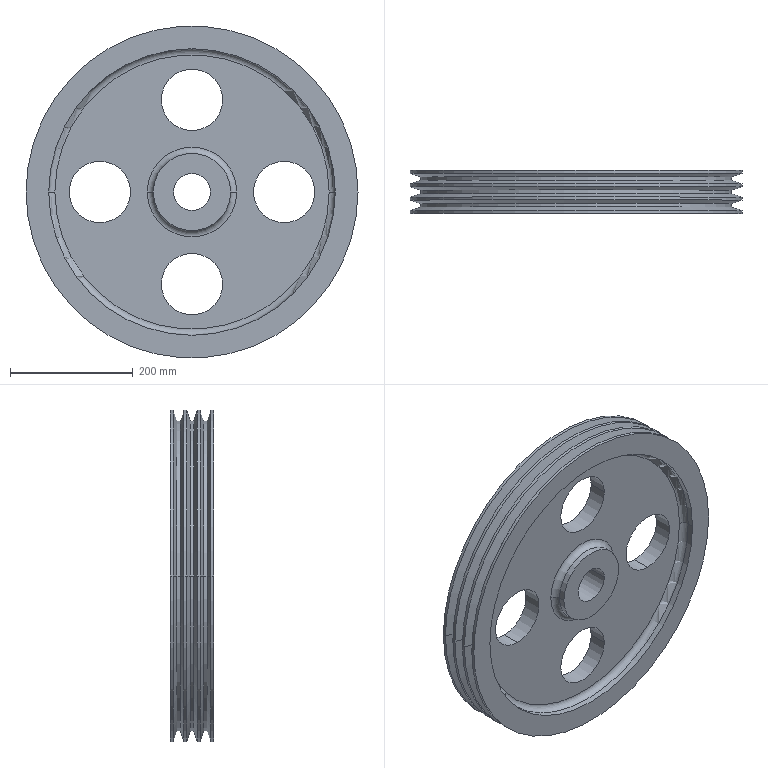Part | Creo | features CUT 4, DATUM PLANE 3, CURVE 2, COORDINATE SYSTEM 1, PATTERN 1, PROTRUSION 1 | 1 solid | 58 faces | box 540 x 70.006 x 540 mm | volume 7681401 mm3 | cylinder 32 | cone 12 | torus 8 | plane 6 | commonest cylinder face diameters 100 x8 540 x8 506 x6 126 x4 466 x4 60 x2
STEP:
#1=CARTESIAN_POINT('',(0.,0.,0.));
#2=DIRECTION('',(0.,0.,1.));
#3=DIRECTION('',(1.,0.,0.));
#4=AXIS2_PLACEMENT_3D('',#1,#2,#3);
#5=CARTESIAN_POINT('',(63.,0.,0.));
#6=VERTEX_POINT('',#5);
#7=CARTESIAN_POINT('',(-63.,0.,0.));
#8=VERTEX_POINT('',#7);
#9=CARTESIAN_POINT('',(0.,0.,0.));
#10=DIRECTION('',(0.,-1.,0.));
#11=DIRECTION('',(1.,0.,0.));
#12=AXIS2_PLACEMENT_3D('',#9,#10,#11);
#13=CIRCLE('',#12,63.);
#14=EDGE_CURVE('',#6,#8,#13,.T.);
#15=ORIENTED_EDGE('',*,*,#14,.F.);
#16=CARTESIAN_POINT('',(0.,0.,0.));
#17=DIRECTION('',(0.,1.,0.));
#18=DIRECTION('',(1.,0.,0.));
#19=AXIS2_PLACEMENT_3D('',#16,#17,#18);
#20=CIRCLE('',#19,63.);
#21=EDGE_CURVE('',#6,#8,#20,.T.);
#22=ORIENTED_EDGE('',*,*,#21,.T.);
#23=EDGE_LOOP('',(#15,#22));
#24=FACE_OUTER_BOUND('',#23,.F.);
#25=CARTESIAN_POINT('',(30.,0.,0.));
#26=VERTEX_POINT('',#25);
#27=CARTESIAN_POINT('',(-30.,0.,0.));
#28=VERTEX_POINT('',#27);
#29=CARTESIAN_POINT('',(0.,0.,0.));
#30=DIRECTION('',(0.,1.,0.));
#31=DIRECTION('',(1.,0.,0.));
#32=AXIS2_PLACEMENT_3D('',#29,#30,#31);
#33=CIRCLE('',#32,30.);
#34=EDGE_CURVE('',#26,#28,#33,.T.);
#35=ORIENTED_EDGE('',*,*,#34,.F.);
#36=CARTESIAN_POINT('',(0.,0.,0.));
#37=DIRECTION('',(0.,-1.,0.));
#38=DIRECTION('',(1.,0.,0.));
#39=AXIS2_PLACEMENT_3D('',#36,#37,#38);
#40=CIRCLE('',#39,30.);
#41=EDGE_CURVE('',#26,#28,#40,.T.);
#42=ORIENTED_EDGE('',*,*,#41,.T.);
#43=EDGE_LOOP('',(#35,#42));
#44=FACE_BOUND('',#43,.F.);
#45=CARTESIAN_POINT('',(0.,0.,0.));
#46=DIRECTION('',(0.,1.,0.));
#47=DIRECTION('',(1.,0.,0.));
#48=AXIS2_PLACEMENT_3D('',#45,#46,#47);
#49=PLANE('',#48);
#50=ADVANCED_FACE('',(#24,#44),#49,.F.);
#51=CARTESIAN_POINT('',(30.,70.006,0.));
#52=VERTEX_POINT('',#51);
#53=CARTESIAN_POINT('',(30.,70.006,0.));
#54=DIRECTION('',(0.,-1.,0.));
#55=VECTOR('',#54,70.006);
#56=LINE('',#53,#55);
#57=EDGE_CURVE('',#52,#26,#56,.T.);
#58=ORIENTED_EDGE('',*,*,#57,.T.);
#59=ORIENTED_EDGE('',*,*,#34,.T.);
#60=CARTESIAN_POINT('',(-30.,70.006,0.));
#61=VERTEX_POINT('',#60);
#62=CARTESIAN_POINT('',(-30.,70.006,0.));
#63=DIRECTION('',(0.,-1.,0.));
#64=VECTOR('',#63,70.006);
#65=LINE('',#62,#64);
#66=EDGE_CURVE('',#61,#28,#65,.T.);
#67=ORIENTED_EDGE('',*,*,#66,.F.);
#68=CARTESIAN_POINT('',(0.,70.006,0.));
#69=DIRECTION('',(0.,1.,0.));
#70=DIRECTION('',(1.,0.,0.));
#71=AXIS2_PLACEMENT_3D('',#68,#69,#70);
#72=CIRCLE('',#71,30.);
#73=EDGE_CURVE('',#52,#61,#72,.T.);
#74=ORIENTED_EDGE('',*,*,#73,.F.);
#75=EDGE_LOOP('',(#58,#59,#67,#74));
#76=FACE_OUTER_BOUND('',#75,.F.);
#77=CARTESIAN_POINT('',(0.,0.,0.));
#78=DIRECTION('',(0.,1.,0.));
#79=DIRECTION('',(1.,0.,0.));
#80=AXIS2_PLACEMENT_3D('',#77,#78,#79);
#81=CYLINDRICAL_SURFACE('',#80,30.);
#82=ADVANCED_FACE('',(#76),#81,.F.);
#83=ORIENTED_EDGE('',*,*,#57,.F.);
#84=CARTESIAN_POINT('',(0.,70.006,0.));
#85=DIRECTION('',(0.,-1.,0.));
#86=DIRECTION('',(1.,0.,0.));
#87=AXIS2_PLACEMENT_3D('',#84,#85,#86);
#88=CIRCLE('',#87,30.);
#89=EDGE_CURVE('',#52,#61,#88,.T.);
#90=ORIENTED_EDGE('',*,*,#89,.T.);
#91=ORIENTED_EDGE('',*,*,#66,.T.);
#92=ORIENTED_EDGE('',*,*,#41,.F.);
#93=EDGE_LOOP('',(#83,#90,#91,#92));
#94=FACE_OUTER_BOUND('',#93,.F.);
#95=CARTESIAN_POINT('',(0.,0.,0.));
#96=DIRECTION('',(0.,1.,0.));
#97=DIRECTION('',(1.,0.,0.));
#98=AXIS2_PLACEMENT_3D('',#95,#96,#97);
#99=CYLINDRICAL_SURFACE('',#98,30.);
#100=ADVANCED_FACE('',(#94),#99,.F.);
#101=CARTESIAN_POINT('',(63.,70.006,0.));
#102=VERTEX_POINT('',#101);
#103=CARTESIAN_POINT('',(-63.,70.006,0.));
#104=VERTEX_POINT('',#103);
#105=CARTESIAN_POINT('',(0.,70.006,0.));
#106=DIRECTION('',(0.,1.,0.));
#107=DIRECTION('',(1.,0.,0.));
#108=AXIS2_PLACEMENT_3D('',#105,#106,#107);
#109=CIRCLE('',#108,63.);
#110=EDGE_CURVE('',#102,#104,#109,.T.);
#111=ORIENTED_EDGE('',*,*,#110,.F.);
#112=CARTESIAN_POINT('',(0.,70.006,0.));
#113=DIRECTION('',(0.,-1.,0.));
#114=DIRECTION('',(1.,0.,0.));
#115=AXIS2_PLACEMENT_3D('',#112,#113,#114);
#116=CIRCLE('',#115,63.);
#117=EDGE_CURVE('',#102,#104,#116,.T.);
#118=ORIENTED_EDGE('',*,*,#117,.T.);
#119=EDGE_LOOP('',(#111,#118));
#120=FACE_OUTER_BOUND('',#119,.F.);
#121=ORIENTED_EDGE('',*,*,#89,.F.);
#122=ORIENTED_EDGE('',*,*,#73,.T.);
#123=EDGE_LOOP('',(#121,#122));
#124=FACE_BOUND('',#123,.F.);
#125=CARTESIAN_POINT('',(0.,70.006,0.));
#126=DIRECTION('',(0.,1.,0.));
#127=DIRECTION('',(1.,0.,0.));
#128=AXIS2_PLACEMENT_3D('',#125,#126,#127);
#129=PLANE('',#128);
#130=ADVANCED_FACE('',(#120,#124),#129,.T.);
#131=CARTESIAN_POINT('',(63.,60.006,0.));
#132=VERTEX_POINT('',#131);
#133=CARTESIAN_POINT('',(63.,60.006,0.));
#134=DIRECTION('',(0.,1.,0.));
#135=VECTOR('',#134,10.);
#136=LINE('',#133,#135);
#137=EDGE_CURVE('',#132,#102,#136,.T.);
#138=ORIENTED_EDGE('',*,*,#137,.T.);
#139=ORIENTED_EDGE('',*,*,#110,.T.);
#140=CARTESIAN_POINT('',(-63.,60.006,0.));
#141=VERTEX_POINT('',#140);
#142=CARTESIAN_POINT('',(-63.,60.006,0.));
#143=DIRECTION('',(0.,1.,0.));
#144=VECTOR('',#143,10.);
#145=LINE('',#142,#144);
#146=EDGE_CURVE('',#141,#104,#145,.T.);
#147=ORIENTED_EDGE('',*,*,#146,.F.);
#148=CARTESIAN_POINT('',(0.,60.006,0.));
#149=DIRECTION('',(0.,1.,0.));
#150=DIRECTION('',(1.,0.,0.));
#151=AXIS2_PLACEMENT_3D('',#148,#149,#150);
#152=CIRCLE('',#151,63.);
#153=EDGE_CURVE('',#132,#141,#152,.T.);
#154=ORIENTED_EDGE('',*,*,#153,.F.);
#155=EDGE_LOOP('',(#138,#139,#147,#154));
#156=FACE_OUTER_BOUND('',#155,.F.);
#157=CARTESIAN_POINT('',(0.,0.,0.));
#158=DIRECTION('',(0.,1.,0.));
#159=DIRECTION('',(1.,0.,0.));
#160=AXIS2_PLACEMENT_3D('',#157,#158,#159);
#161=CYLINDRICAL_SURFACE('',#160,63.);
#162=ADVANCED_FACE('',(#156),#161,.T.);
#163=ORIENTED_EDGE('',*,*,#137,.F.);
#164=CARTESIAN_POINT('',(0.,60.006,0.));
#165=DIRECTION('',(0.,-1.,0.));
#166=DIRECTION('',(1.,0.,0.));
#167=AXIS2_PLACEMENT_3D('',#164,#165,#166);
#168=CIRCLE('',#167,63.);
#169=EDGE_CURVE('',#132,#141,#168,.T.);
#170=ORIENTED_EDGE('',*,*,#169,.T.);
#171=ORIENTED_EDGE('',*,*,#146,.T.);
#172=ORIENTED_EDGE('',*,*,#117,.F.);
#173=EDGE_LOOP('',(#163,#170,#171,#172));
#174=FACE_OUTER_BOUND('',#173,.F.);
#175=CARTESIAN_POINT('',(0.,0.,0.));
#176=DIRECTION('',(0.,1.,0.));
#177=DIRECTION('',(1.,0.,0.));
#178=AXIS2_PLACEMENT_3D('',#175,#176,#177);
#179=CYLINDRICAL_SURFACE('',#178,63.);
#180=ADVANCED_FACE('',(#174),#179,.T.);
#181=CARTESIAN_POINT('',(73.,50.006,0.));
#182=VERTEX_POINT('',#181);
#183=CARTESIAN_POINT('',(73.,60.006,0.));
#184=DIRECTION('',(0.,0.,-1.));
#185=DIRECTION('',(0.,-1.,0.));
#186=AXIS2_PLACEMENT_3D('',#183,#184,#185);
#187=CIRCLE('',#186,10.);
#188=EDGE_CURVE('',#182,#132,#187,.T.);
#189=ORIENTED_EDGE('',*,*,#188,.F.);
#190=CARTESIAN_POINT('',(-73.,50.006,0.));
#191=VERTEX_POINT('',#190);
#192=CARTESIAN_POINT('',(0.,50.006,0.));
#193=DIRECTION('',(0.,-1.,0.));
#194=DIRECTION('',(1.,0.,0.));
#195=AXIS2_PLACEMENT_3D('',#192,#193,#194);
#196=CIRCLE('',#195,73.);
#197=EDGE_CURVE('',#182,#191,#196,.T.);
#198=ORIENTED_EDGE('',*,*,#197,.T.);
#199=CARTESIAN_POINT('',(-73.,60.006,0.));
#200=DIRECTION('',(0.,0.,1.));
#201=DIRECTION('',(0.,-1.,0.));
#202=AXIS2_PLACEMENT_3D('',#199,#200,#201);
#203=CIRCLE('',#202,10.);
#204=EDGE_CURVE('',#191,#141,#203,.T.);
#205=ORIENTED_EDGE('',*,*,#204,.T.);
#206=ORIENTED_EDGE('',*,*,#169,.F.);
#207=EDGE_LOOP('',(#189,#198,#205,#206));
#208=FACE_OUTER_BOUND('',#207,.F.);
#209=CARTESIAN_POINT('',(0.,60.006,0.));
#210=DIRECTION('',(0.,1.,0.));
#211=DIRECTION('',(1.,0.,0.));
#212=AXIS2_PLACEMENT_3D('',#209,#210,#211);
#213=TOROIDAL_SURFACE('',#212,73.,10.);
#214=ADVANCED_FACE('',(#208),#213,.F.);
#215=ORIENTED_EDGE('',*,*,#188,.T.);
#216=ORIENTED_EDGE('',*,*,#153,.T.);
#217=ORIENTED_EDGE('',*,*,#204,.F.);
#218=CARTESIAN_POINT('',(0.,50.006,0.));
#219=DIRECTION('',(0.,1.,0.));
#220=DIRECTION('',(1.,0.,0.));
#221=AXIS2_PLACEMENT_3D('',#218,#219,#220);
#222=CIRCLE('',#221,73.);
#223=EDGE_CURVE('',#182,#191,#222,.T.);
#224=ORIENTED_EDGE('',*,*,#223,.F.);
#225=EDGE_LOOP('',(#215,#216,#217,#224));
#226=FACE_OUTER_BOUND('',#225,.F.);
#227=CARTESIAN_POINT('',(0.,60.006,0.));
#228=DIRECTION('',(0.,1.,0.));
#229=DIRECTION('',(1.,0.,0.));
#230=AXIS2_PLACEMENT_3D('',#227,#228,#229);
#231=TOROIDAL_SURFACE('',#230,73.,10.);
#232=ADVANCED_FACE('',(#226),#231,.F.);
#233=CARTESIAN_POINT('',(223.,50.006,0.));
#234=VERTEX_POINT('',#233);
#235=CARTESIAN_POINT('',(-223.,50.006,0.));
#236=VERTEX_POINT('',#235);
#237=CARTESIAN_POINT('',(0.,50.006,0.));
#238=DIRECTION('',(0.,1.,0.));
#239=DIRECTION('',(1.,0.,0.));
#240=AXIS2_PLACEMENT_3D('',#237,#238,#239);
#241=CIRCLE('',#240,223.);
#242=EDGE_CURVE('',#234,#236,#241,.T.);
#243=ORIENTED_EDGE('',*,*,#242,.F.);
#244=CARTESIAN_POINT('',(0.,50.006,0.));
#245=DIRECTION('',(0.,-1.,0.));
#246=DIRECTION('',(1.,0.,0.));
#247=AXIS2_PLACEMENT_3D('',#244,#245,#246);
#248=CIRCLE('',#247,223.);
#249=EDGE_CURVE('',#234,#236,#248,.T.);
#250=ORIENTED_EDGE('',*,*,#249,.T.);
#251=EDGE_LOOP('',(#243,#250));
#252=FACE_OUTER_BOUND('',#251,.F.);
#253=ORIENTED_EDGE('',*,*,#197,.F.);
#254=ORIENTED_EDGE('',*,*,#223,.T.);
#255=EDGE_LOOP('',(#253,#254));
#256=FACE_BOUND('',#255,.F.);
#257=CARTESIAN_POINT('',(150.,50.006,50.));
#258=VERTEX_POINT('',#257);
#259=CARTESIAN_POINT('',(150.,50.006,-50.));
#260=VERTEX_POINT('',#259);
#261=CARTESIAN_POINT('',(150.,50.006,0.));
#262=DIRECTION('',(0.,1.,0.));
#263=DIRECTION('',(0.,0.,1.));
#264=AXIS2_PLACEMENT_3D('',#261,#262,#263);
#265=CIRCLE('',#264,50.);
#266=EDGE_CURVE('',#258,#260,#265,.T.);
#267=ORIENTED_EDGE('',*,*,#266,.T.);
#268=CARTESIAN_POINT('',(150.,50.006,0.));
#269=DIRECTION('',(0.,1.,0.));
#270=DIRECTION('',(0.,0.,-1.));
#271=AXIS2_PLACEMENT_3D('',#268,#269,#270);
#272=CIRCLE('',#271,50.);
#273=EDGE_CURVE('',#260,#258,#272,.T.);
#274=ORIENTED_EDGE('',*,*,#273,.T.);
#275=EDGE_LOOP('',(#267,#274));
#276=FACE_BOUND('',#275,.F.);
#277=CARTESIAN_POINT('',(50.,50.006,-150.));
#278=VERTEX_POINT('',#277);
#279=CARTESIAN_POINT('',(-50.,50.006,-150.));
#280=VERTEX_POINT('',#279);
#281=CARTESIAN_POINT('',(0.,50.006,-150.));
#282=DIRECTION('',(0.,1.,0.));
#283=DIRECTION('',(1.,0.,0.));
#284=AXIS2_PLACEMENT_3D('',#281,#282,#283);
#285=CIRCLE('',#284,50.);
#286=EDGE_CURVE('',#278,#280,#285,.T.);
#287=ORIENTED_EDGE('',*,*,#286,.T.);
#288=CARTESIAN_POINT('',(0.,50.006,-150.));
#289=DIRECTION('',(0.,1.,0.));
#290=DIRECTION('',(-1.,0.,0.));
#291=AXIS2_PLACEMENT_3D('',#288,#289,#290);
#292=CIRCLE('',#291,50.);
#293=EDGE_CURVE('',#280,#278,#292,.T.);
#294=ORIENTED_EDGE('',*,*,#293,.T.);
#295=EDGE_LOOP('',(#287,#294));
#296=FACE_BOUND('',#295,.F.);
#297=CARTESIAN_POINT('',(-150.,50.006,-50.));
#298=VERTEX_POINT('',#297);
#299=CARTESIAN_POINT('',(-150.,50.006,50.));
#300=VERTEX_POINT('',#299);
#301=CARTESIAN_POINT('',(-150.,50.006,0.));
#302=DIRECTION('',(0.,1.,0.));
#303=DIRECTION('',(0.,0.,-1.));
#304=AXIS2_PLACEMENT_3D('',#301,#302,#303);
#305=CIRCLE('',#304,50.);
#306=EDGE_CURVE('',#298,#300,#305,.T.);
#307=ORIENTED_EDGE('',*,*,#306,.T.);
#308=CARTESIAN_POINT('',(-150.,50.006,0.));
#309=DIRECTION('',(0.,1.,0.));
#310=DIRECTION('',(0.,0.,1.));
#311=AXIS2_PLACEMENT_3D('',#308,#309,#310);
#312=CIRCLE('',#311,50.);
#313=EDGE_CURVE('',#300,#298,#312,.T.);
#314=ORIENTED_EDGE('',*,*,#313,.T.);
#315=EDGE_LOOP('',(#307,#314));
#316=FACE_BOUND('',#315,.F.);
#317=CARTESIAN_POINT('',(-50.,50.006,150.));
#318=VERTEX_POINT('',#317);
#319=CARTESIAN_POINT('',(50.,50.006,150.));
#320=VERTEX_POINT('',#319);
#321=CARTESIAN_POINT('',(0.,50.006,150.));
#322=DIRECTION('',(0.,1.,0.));
#323=DIRECTION('',(-1.,0.,0.));
#324=AXIS2_PLACEMENT_3D('',#321,#322,#323);
#325=CIRCLE('',#324,50.);
#326=EDGE_CURVE('',#318,#320,#325,.T.);
#327=ORIENTED_EDGE('',*,*,#326,.T.);
#328=CARTESIAN_POINT('',(0.,50.006,150.));
#329=DIRECTION('',(0.,1.,0.));
#330=DIRECTION('',(1.,0.,0.));
#331=AXIS2_PLACEMENT_3D('',#328,#329,#330);
#332=CIRCLE('',#331,50.);
#333=EDGE_CURVE('',#320,#318,#332,.T.);
#334=ORIENTED_EDGE('',*,*,#333,.T.);
#335=EDGE_LOOP('',(#327,#334));
#336=FACE_BOUND('',#335,.F.);
#337=CARTESIAN_POINT('',(0.,50.006,0.));
#338=DIRECTION('',(0.,1.,0.));
#339=DIRECTION('',(1.,0.,0.));
#340=AXIS2_PLACEMENT_3D('',#337,#338,#339);
#341=PLANE('',#340);
#342=ADVANCED_FACE('',(#252,#256,#276,#296,#316,#336),#341,.T.);
#343=CARTESIAN_POINT('',(233.,60.006,0.));
#344=VERTEX_POINT('',#343);
#345=CARTESIAN_POINT('',(223.,60.006,0.));
#346=DIRECTION('',(0.,0.,-1.));
#347=DIRECTION('',(1.,0.,0.));
#348=AXIS2_PLACEMENT_3D('',#345,#346,#347);
#349=CIRCLE('',#348,10.);
#350=EDGE_CURVE('',#344,#234,#349,.T.);
#351=ORIENTED_EDGE('',*,*,#350,.T.);
#352=ORIENTED_EDGE('',*,*,#242,.T.);
#353=CARTESIAN_POINT('',(-233.,60.006,0.));
#354=VERTEX_POINT('',#353);
#355=CARTESIAN_POINT('',(-223.,60.006,0.));
#356=DIRECTION('',(0.,0.,1.));
#357=DIRECTION('',(-1.,0.,0.));
#358=AXIS2_PLACEMENT_3D('',#355,#356,#357);
#359=CIRCLE('',#358,10.);
#360=EDGE_CURVE('',#354,#236,#359,.T.);
#361=ORIENTED_EDGE('',*,*,#360,.F.);
#362=CARTESIAN_POINT('',(0.,60.006,0.));
#363=DIRECTION('',(0.,1.,0.));
#364=DIRECTION('',(1.,0.,0.));
#365=AXIS2_PLACEMENT_3D('',#362,#363,#364);
#366=CIRCLE('',#365,233.);
#367=EDGE_CURVE('',#344,#354,#366,.T.);
#368=ORIENTED_EDGE('',*,*,#367,.F.);
#369=EDGE_LOOP('',(#351,#352,#361,#368));
#370=FACE_OUTER_BOUND('',#369,.F.);
#371=CARTESIAN_POINT('',(0.,60.006,0.));
#372=DIRECTION('',(0.,1.,0.));
#373=DIRECTION('',(1.,0.,0.));
#374=AXIS2_PLACEMENT_3D('',#371,#372,#373);
#375=TOROIDAL_SURFACE('',#374,223.,10.);
#376=ADVANCED_FACE('',(#370),#375,.F.);
#377=ORIENTED_EDGE('',*,*,#350,.F.);
#378=CARTESIAN_POINT('',(0.,60.006,0.));
#379=DIRECTION('',(0.,-1.,0.));
#380=DIRECTION('',(1.,0.,0.));
#381=AXIS2_PLACEMENT_3D('',#378,#379,#380);
#382=CIRCLE('',#381,233.);
#383=EDGE_CURVE('',#344,#354,#382,.T.);
#384=ORIENTED_EDGE('',*,*,#383,.T.);
#385=ORIENTED_EDGE('',*,*,#360,.T.);
#386=ORIENTED_EDGE('',*,*,#249,.F.);
#387=EDGE_LOOP('',(#377,#384,#385,#386));
#388=FACE_OUTER_BOUND('',#387,.F.);
#389=CARTESIAN_POINT('',(0.,60.006,0.));
#390=DIRECTION('',(0.,1.,0.));
#391=DIRECTION('',(1.,0.,0.));
#392=AXIS2_PLACEMENT_3D('',#389,#390,#391);
#393=TOROIDAL_SURFACE('',#392,223.,10.);
#394=ADVANCED_FACE('',(#388),#393,.F.);
#395=CARTESIAN_POINT('',(233.,70.006,0.));
#396=VERTEX_POINT('',#395);
#397=CARTESIAN_POINT('',(233.,70.006,0.));
#398=DIRECTION('',(0.,-1.,0.));
#399=VECTOR('',#398,10.);
#400=LINE('',#397,#399);
#401=EDGE_CURVE('',#396,#344,#400,.T.);
#402=ORIENTED_EDGE('',*,*,#401,.F.);
#403=CARTESIAN_POINT('',(-233.,70.006,0.));
#404=VERTEX_POINT('',#403);
#405=CARTESIAN_POINT('',(0.,70.006,0.));
#406=DIRECTION('',(0.,-1.,0.));
#407=DIRECTION('',(1.,0.,0.));
#408=AXIS2_PLACEMENT_3D('',#405,#406,#407);
#409=CIRCLE('',#408,233.);
#410=EDGE_CURVE('',#396,#404,#409,.T.);
#411=ORIENTED_EDGE('',*,*,#410,.T.);
#412=CARTESIAN_POINT('',(-233.,70.006,0.));
#413=DIRECTION('',(0.,-1.,0.));
#414=VECTOR('',#413,10.);
#415=LINE('',#412,#414);
#416=EDGE_CURVE('',#404,#354,#415,.T.);
#417=ORIENTED_EDGE('',*,*,#416,.T.);
#418=ORIENTED_EDGE('',*,*,#383,.F.);
#419=EDGE_LOOP('',(#402,#411,#417,#418));
#420=FACE_OUTER_BOUND('',#419,.F.);
#421=CARTESIAN_POINT('',(0.,0.,0.));
#422=DIRECTION('',(0.,1.,0.));
#423=DIRECTION('',(1.,0.,0.));
#424=AXIS2_PLACEMENT_3D('',#421,#422,#423);
#425=CYLINDRICAL_SURFACE('',#424,233.);
#426=ADVANCED_FACE('',(#420),#425,.F.);
#427=ORIENTED_EDGE('',*,*,#401,.T.);
#428=ORIENTED_EDGE('',*,*,#367,.T.);
#429=ORIENTED_EDGE('',*,*,#416,.F.);
#430=CARTESIAN_POINT('',(0.,70.006,0.));
#431=DIRECTION('',(0.,1.,0.));
#432=DIRECTION('',(1.,0.,0.));
#433=AXIS2_PLACEMENT_3D('',#430,#431,#432);
#434=CIRCLE('',#433,233.);
#435=EDGE_CURVE('',#396,#404,#434,.T.);
#436=ORIENTED_EDGE('',*,*,#435,.F.);
#437=EDGE_LOOP('',(#427,#428,#429,#436));
#438=FACE_OUTER_BOUND('',#437,.F.);
#439=CARTESIAN_POINT('',(0.,0.,0.));
#440=DIRECTION('',(0.,1.,0.));
#441=DIRECTION('',(1.,0.,0.));
#442=AXIS2_PLACEMENT_3D('',#439,#440,#441);
#443=CYLINDRICAL_SURFACE('',#442,233.);
#444=ADVANCED_FACE('',(#438),#443,.F.);
#445=CARTESIAN_POINT('',(270.,70.006,0.));
#446=VERTEX_POINT('',#445);
#447=CARTESIAN_POINT('',(-270.,70.006,0.));
#448=VERTEX_POINT('',#447);
#449=CARTESIAN_POINT('',(0.,70.006,0.));
#450=DIRECTION('',(0.,1.,0.));
#451=DIRECTION('',(1.,0.,0.));
#452=AXIS2_PLACEMENT_3D('',#449,#450,#451);
#453=CIRCLE('',#452,270.);
#454=EDGE_CURVE('',#446,#448,#453,.T.);
#455=ORIENTED_EDGE('',*,*,#454,.F.);
#456=CARTESIAN_POINT('',(0.,70.006,0.));
#457=DIRECTION('',(0.,-1.,0.));
#458=DIRECTION('',(1.,0.,0.));
#459=AXIS2_PLACEMENT_3D('',#456,#457,#458);
#460=CIRCLE('',#459,270.);
#461=EDGE_CURVE('',#446,#448,#460,.T.);
#462=ORIENTED_EDGE('',*,*,#461,.T.);
#463=EDGE_LOOP('',(#455,#462));
#464=FACE_OUTER_BOUND('',#463,.F.);
#465=ORIENTED_EDGE('',*,*,#410,.F.);
#466=ORIENTED_EDGE('',*,*,#435,.T.);
#467=EDGE_LOOP('',(#465,#466));
#468=FACE_BOUND('',#467,.F.);
#469=CARTESIAN_POINT('',(0.,70.006,0.));
#470=DIRECTION('',(0.,1.,0.));
#471=DIRECTION('',(1.,0.,0.));
#472=AXIS2_PLACEMENT_3D('',#469,#470,#471);
#473=PLANE('',#472);
#474=ADVANCED_FACE('',(#464,#468),#473,.T.);
#475=CARTESIAN_POINT('',(270.,65.256,0.));
#476=VERTEX_POINT('',#475);
#477=CARTESIAN_POINT('',(270.,65.256,0.));
#478=DIRECTION('',(0.,1.,0.));
#479=VECTOR('',#478,4.75);
#480=LINE('',#477,#479);
#481=EDGE_CURVE('',#476,#446,#480,.T.);
#482=ORIENTED_EDGE('',*,*,#481,.T.);
#483=ORIENTED_EDGE('',*,*,#454,.T.);
#484=CARTESIAN_POINT('',(-270.,65.256,0.));
#485=VERTEX_POINT('',#484);
#486=CARTESIAN_POINT('',(-270.,65.256,0.));
#487=DIRECTION('',(0.,1.,0.));
#488=VECTOR('',#487,4.75);
#489=LINE('',#486,#488);
#490=EDGE_CURVE('',#485,#448,#489,.T.);
#491=ORIENTED_EDGE('',*,*,#490,.F.);
#492=CARTESIAN_POINT('',(0.,65.256,0.));
#493=DIRECTION('',(0.,1.,0.));
#494=DIRECTION('',(1.,0.,0.));
#495=AXIS2_PLACEMENT_3D('',#492,#493,#494);
#496=CIRCLE('',#495,270.);
#497=EDGE_CURVE('',#476,#485,#496,.T.);
#498=ORIENTED_EDGE('',*,*,#497,.F.);
#499=EDGE_LOOP('',(#482,#483,#491,#498));
#500=FACE_OUTER_BOUND('',#499,.F.);
#501=CARTESIAN_POINT('',(0.,0.,0.));
#502=DIRECTION('',(0.,1.,0.));
#503=DIRECTION('',(1.,0.,0.));
#504=AXIS2_PLACEMENT_3D('',#501,#502,#503);
#505=CYLINDRICAL_SURFACE('',#504,270.);
#506=ADVANCED_FACE('',(#500),#505,.T.);
#507=ORIENTED_EDGE('',*,*,#481,.F.);
#508=CARTESIAN_POINT('',(0.,65.256,0.));
#509=DIRECTION('',(0.,-1.,0.));
#510=DIRECTION('',(1.,0.,0.));
#511=AXIS2_PLACEMENT_3D('',#508,#509,#510);
#512=CIRCLE('',#511,270.);
#513=EDGE_CURVE('',#476,#485,#512,.T.);
#514=ORIENTED_EDGE('',*,*,#513,.T.);
#515=ORIENTED_EDGE('',*,*,#490,.T.);
#516=ORIENTED_EDGE('',*,*,#461,.F.);
#517=EDGE_LOOP('',(#507,#514,#515,#516));
#518=FACE_OUTER_BOUND('',#517,.F.);
#519=CARTESIAN_POINT('',(0.,0.,0.));
#520=DIRECTION('',(0.,1.,0.));
#521=DIRECTION('',(1.,0.,0.));
#522=AXIS2_PLACEMENT_3D('',#519,#520,#521);
#523=CYLINDRICAL_SURFACE('',#522,270.);
#524=ADVANCED_FACE('',(#518),#523,.T.);
#525=CARTESIAN_POINT('',(253.,59.732,0.));
#526=VERTEX_POINT('',#525);
#527=CARTESIAN_POINT('',(253.,59.732,0.));
#528=DIRECTION('',(0.9511,0.309,0.));
#529=VECTOR('',#528,17.875);
#530=LINE('',#527,#529);
#531=EDGE_CURVE('',#526,#476,#530,.T.);
#532=ORIENTED_EDGE('',*,*,#531,.F.);
#533=CARTESIAN_POINT('',(-253.,59.732,0.));
#534=VERTEX_POINT('',#533);
#535=CARTESIAN_POINT('',(0.,59.732,0.));
#536=DIRECTION('',(0.,-1.,0.));
#537=DIRECTION('',(1.,0.,0.));
#538=AXIS2_PLACEMENT_3D('',#535,#536,#537);
#539=CIRCLE('',#538,253.);
#540=EDGE_CURVE('',#526,#534,#539,.T.);
#541=ORIENTED_EDGE('',*,*,#540,.T.);
#542=CARTESIAN_POINT('',(-253.,59.732,0.));
#543=DIRECTION('',(-0.9511,0.309,0.));
#544=VECTOR('',#543,17.875);
#545=LINE('',#542,#544);
#546=EDGE_CURVE('',#534,#485,#545,.T.);
#547=ORIENTED_EDGE('',*,*,#546,.T.);
#548=ORIENTED_EDGE('',*,*,#513,.F.);
#549=EDGE_LOOP('',(#532,#541,#547,#548));
#550=FACE_OUTER_BOUND('',#549,.F.);
#551=CARTESIAN_POINT('',(0.,62.494,0.));
#552=DIRECTION('',(0.,1.,0.));
#553=DIRECTION('',(1.,0.,0.));
#554=AXIS2_PLACEMENT_3D('',#551,#552,#553);
#555=CONICAL_SURFACE('',#554,261.5,72.);
#556=ADVANCED_FACE('',(#550),#555,.T.);
#557=ORIENTED_EDGE('',*,*,#531,.T.);
#558=ORIENTED_EDGE('',*,*,#497,.T.);
#559=ORIENTED_EDGE('',*,*,#546,.F.);
#560=CARTESIAN_POINT('',(0.,59.732,0.));
#561=DIRECTION('',(0.,1.,0.));
#562=DIRECTION('',(1.,0.,0.));
#563=AXIS2_PLACEMENT_3D('',#560,#561,#562);
#564=CIRCLE('',#563,253.);
#565=EDGE_CURVE('',#526,#534,#564,.T.);
#566=ORIENTED_EDGE('',*,*,#565,.F.);
#567=EDGE_LOOP('',(#557,#558,#559,#566));
#568=FACE_OUTER_BOUND('',#567,.F.);
#569=CARTESIAN_POINT('',(0.,62.494,0.));
#570=DIRECTION('',(0.,1.,0.));
#571=DIRECTION('',(1.,0.,0.));
#572=AXIS2_PLACEMENT_3D('',#569,#570,#571);
#573=CONICAL_SURFACE('',#572,261.5,72.);
#574=ADVANCED_FACE('',(#568),#573,.T.);
#575=CARTESIAN_POINT('',(253.,53.772,0.));
#576=VERTEX_POINT('',#575);
#577=CARTESIAN_POINT('',(253.,53.772,0.));
#578=DIRECTION('',(0.,1.,0.));
#579=VECTOR('',#578,5.96);
#580=LINE('',#577,#579);
#581=EDGE_CURVE('',#576,#526,#580,.T.);
#582=ORIENTED_EDGE('',*,*,#581,.T.);
#583=ORIENTED_EDGE('',*,*,#565,.T.);
#584=CARTESIAN_POINT('',(-253.,53.772,0.));
#585=VERTEX_POINT('',#584);
#586=CARTESIAN_POINT('',(-253.,53.772,0.));
#587=DIRECTION('',(0.,1.,0.));
#588=VECTOR('',#587,5.96);
#589=LINE('',#586,#588);
#590=EDGE_CURVE('',#585,#534,#589,.T.);
#591=ORIENTED_EDGE('',*,*,#590,.F.);
#592=CARTESIAN_POINT('',(0.,53.772,0.));
#593=DIRECTION('',(0.,1.,0.));
#594=DIRECTION('',(1.,0.,0.));
#595=AXIS2_PLACEMENT_3D('',#592,#593,#594);
#596=CIRCLE('',#595,253.);
#597=EDGE_CURVE('',#576,#585,#596,.T.);
#598=ORIENTED_EDGE('',*,*,#597,.F.);
#599=EDGE_LOOP('',(#582,#583,#591,#598));
#600=FACE_OUTER_BOUND('',#599,.F.);
#601=CARTESIAN_POINT('',(0.,0.,0.));
#602=DIRECTION('',(0.,1.,0.));
#603=DIRECTION('',(1.,0.,0.));
#604=AXIS2_PLACEMENT_3D('',#601,#602,#603);
#605=CYLINDRICAL_SURFACE('',#604,253.);
#606=ADVANCED_FACE('',(#600),#605,.T.);
#607=ORIENTED_EDGE('',*,*,#581,.F.);
#608=CARTESIAN_POINT('',(0.,53.772,0.));
#609=DIRECTION('',(0.,-1.,0.));
#610=DIRECTION('',(1.,0.,0.));
#611=AXIS2_PLACEMENT_3D('',#608,#609,#610);
#612=CIRCLE('',#611,253.);
#613=EDGE_CURVE('',#576,#585,#612,.T.);
#614=ORIENTED_EDGE('',*,*,#613,.T.);
#615=ORIENTED_EDGE('',*,*,#590,.T.);
#616=ORIENTED_EDGE('',*,*,#540,.F.);
#617=EDGE_LOOP('',(#607,#614,#615,#616));
#618=FACE_OUTER_BOUND('',#617,.F.);
#619=CARTESIAN_POINT('',(0.,0.,0.));
#620=DIRECTION('',(0.,1.,0.));
#621=DIRECTION('',(1.,0.,0.));
#622=AXIS2_PLACEMENT_3D('',#619,#620,#621);
#623=CYLINDRICAL_SURFACE('',#622,253.);
#624=ADVANCED_FACE('',(#618),#623,.T.);
#625=CARTESIAN_POINT('',(270.,48.248,0.));
#626=VERTEX_POINT('',#625);
#627=CARTESIAN_POINT('',(270.,48.248,0.));
#628=DIRECTION('',(-0.9511,0.309,0.));
#629=VECTOR('',#628,17.875);
#630=LINE('',#627,#629);
#631=EDGE_CURVE('',#626,#576,#630,.T.);
#632=ORIENTED_EDGE('',*,*,#631,.F.);
#633=CARTESIAN_POINT('',(-270.,48.248,0.));
#634=VERTEX_POINT('',#633);
#635=CARTESIAN_POINT('',(0.,48.248,0.));
#636=DIRECTION('',(0.,-1.,0.));
#637=DIRECTION('',(1.,0.,0.));
#638=AXIS2_PLACEMENT_3D('',#635,#636,#637);
#639=CIRCLE('',#638,270.);
#640=EDGE_CURVE('',#626,#634,#639,.T.);
#641=ORIENTED_EDGE('',*,*,#640,.T.);
#642=CARTESIAN_POINT('',(-270.,48.248,0.));
#643=DIRECTION('',(0.9511,0.309,0.));
#644=VECTOR('',#643,17.875);
#645=LINE('',#642,#644);
#646=EDGE_CURVE('',#634,#585,#645,.T.);
#647=ORIENTED_EDGE('',*,*,#646,.T.);
#648=ORIENTED_EDGE('',*,*,#613,.F.);
#649=EDGE_LOOP('',(#632,#641,#647,#648));
#650=FACE_OUTER_BOUND('',#649,.F.);
#651=CARTESIAN_POINT('',(0.,51.01,0.));
#652=DIRECTION('',(0.,-1.,0.));
#653=DIRECTION('',(-1.,0.,0.));
#654=AXIS2_PLACEMENT_3D('',#651,#652,#653);
#655=CONICAL_SURFACE('',#654,261.5,72.);
#656=ADVANCED_FACE('',(#650),#655,.T.);
#657=ORIENTED_EDGE('',*,*,#631,.T.);
#658=ORIENTED_EDGE('',*,*,#597,.T.);
#659=ORIENTED_EDGE('',*,*,#646,.F.);
#660=CARTESIAN_POINT('',(0.,48.248,0.));
#661=DIRECTION('',(0.,1.,0.));
#662=DIRECTION('',(1.,0.,0.));
#663=AXIS2_PLACEMENT_3D('',#660,#661,#662);
#664=CIRCLE('',#663,270.);
#665=EDGE_CURVE('',#626,#634,#664,.T.);
#666=ORIENTED_EDGE('',*,*,#665,.F.);
#667=EDGE_LOOP('',(#657,#658,#659,#666));
#668=FACE_OUTER_BOUND('',#667,.F.);
#669=CARTESIAN_POINT('',(0.,51.01,0.));
#670=DIRECTION('',(0.,-1.,0.));
#671=DIRECTION('',(-1.,0.,0.));
#672=AXIS2_PLACEMENT_3D('',#669,#670,#671);
#673=CONICAL_SURFACE('',#672,261.5,72.);
#674=ADVANCED_FACE('',(#668),#673,.T.);
#675=CARTESIAN_POINT('',(270.,43.512,0.));
#676=VERTEX_POINT('',#675);
#677=CARTESIAN_POINT('',(270.,43.512,0.));
#678=DIRECTION('',(0.,1.,0.));
#679=VECTOR('',#678,4.737);
#680=LINE('',#677,#679);
#681=EDGE_CURVE('',#676,#626,#680,.T.);
#682=ORIENTED_EDGE('',*,*,#681,.T.);
#683=ORIENTED_EDGE('',*,*,#665,.T.);
#684=CARTESIAN_POINT('',(-270.,43.512,0.));
#685=VERTEX_POINT('',#684);
#686=CARTESIAN_POINT('',(-270.,43.512,0.));
#687=DIRECTION('',(0.,1.,0.));
#688=VECTOR('',#687,4.737);
#689=LINE('',#686,#688);
#690=EDGE_CURVE('',#685,#634,#689,.T.);
#691=ORIENTED_EDGE('',*,*,#690,.F.);
#692=CARTESIAN_POINT('',(0.,43.512,0.));
#693=DIRECTION('',(0.,1.,0.));
#694=DIRECTION('',(1.,0.,0.));
#695=AXIS2_PLACEMENT_3D('',#692,#693,#694);
#696=CIRCLE('',#695,270.);
#697=EDGE_CURVE('',#676,#685,#696,.T.);
#698=ORIENTED_EDGE('',*,*,#697,.F.);
#699=EDGE_LOOP('',(#682,#683,#691,#698));
#700=FACE_OUTER_BOUND('',#699,.F.);
#701=CARTESIAN_POINT('',(0.,0.,0.));
#702=DIRECTION('',(0.,1.,0.));
#703=DIRECTION('',(1.,0.,0.));
#704=AXIS2_PLACEMENT_3D('',#701,#702,#703);
#705=CYLINDRICAL_SURFACE('',#704,270.);
#706=ADVANCED_FACE('',(#700),#705,.T.);
#707=ORIENTED_EDGE('',*,*,#681,.F.);
#708=CARTESIAN_POINT('',(0.,43.512,0.));
#709=DIRECTION('',(0.,-1.,0.));
#710=DIRECTION('',(1.,0.,0.));
#711=AXIS2_PLACEMENT_3D('',#708,#709,#710);
#712=CIRCLE('',#711,270.);
#713=EDGE_CURVE('',#676,#685,#712,.T.);
#714=ORIENTED_EDGE('',*,*,#713,.T.);
#715=ORIENTED_EDGE('',*,*,#690,.T.);
#716=ORIENTED_EDGE('',*,*,#640,.F.);
#717=EDGE_LOOP('',(#707,#714,#715,#716));
#718=FACE_OUTER_BOUND('',#717,.F.);
#719=CARTESIAN_POINT('',(0.,0.,0.));
#720=DIRECTION('',(0.,1.,0.));
#721=DIRECTION('',(1.,0.,0.));
#722=AXIS2_PLACEMENT_3D('',#719,#720,#721);
#723=CYLINDRICAL_SURFACE('',#722,270.);
#724=ADVANCED_FACE('',(#718),#723,.T.);
#725=CARTESIAN_POINT('',(253.,37.988,0.));
#726=VERTEX_POINT('',#725);
#727=CARTESIAN_POINT('',(253.,37.988,0.));
#728=DIRECTION('',(0.9511,0.309,0.));
#729=VECTOR('',#728,17.875);
#730=LINE('',#727,#729);
#731=EDGE_CURVE('',#726,#676,#730,.T.);
#732=ORIENTED_EDGE('',*,*,#731,.F.);
#733=CARTESIAN_POINT('',(-253.,37.988,0.));
#734=VERTEX_POINT('',#733);
#735=CARTESIAN_POINT('',(0.,37.988,0.));
#736=DIRECTION('',(0.,-1.,0.));
#737=DIRECTION('',(1.,0.,0.));
#738=AXIS2_PLACEMENT_3D('',#735,#736,#737);
#739=CIRCLE('',#738,253.);
#740=EDGE_CURVE('',#726,#734,#739,.T.);
#741=ORIENTED_EDGE('',*,*,#740,.T.);
#742=CARTESIAN_POINT('',(-253.,37.988,0.));
#743=DIRECTION('',(-0.9511,0.309,0.));
#744=VECTOR('',#743,17.875);
#745=LINE('',#742,#744);
#746=EDGE_CURVE('',#734,#685,#745,.T.);
#747=ORIENTED_EDGE('',*,*,#746,.T.);
#748=ORIENTED_EDGE('',*,*,#713,.F.);
#749=EDGE_LOOP('',(#732,#741,#747,#748));
#750=FACE_OUTER_BOUND('',#749,.F.);
#751=CARTESIAN_POINT('',(0.,40.75,0.));
#752=DIRECTION('',(0.,1.,0.));
#753=DIRECTION('',(1.,0.,0.));
#754=AXIS2_PLACEMENT_3D('',#751,#752,#753);
#755=CONICAL_SURFACE('',#754,261.5,72.);
#756=ADVANCED_FACE('',(#750),#755,.T.);
#757=ORIENTED_EDGE('',*,*,#731,.T.);
#758=ORIENTED_EDGE('',*,*,#697,.T.);
#759=ORIENTED_EDGE('',*,*,#746,.F.);
#760=CARTESIAN_POINT('',(0.,37.988,0.));
#761=DIRECTION('',(0.,1.,0.));
#762=DIRECTION('',(1.,0.,0.));
#763=AXIS2_PLACEMENT_3D('',#760,#761,#762);
#764=CIRCLE('',#763,253.);
#765=EDGE_CURVE('',#726,#734,#764,.T.);
#766=ORIENTED_EDGE('',*,*,#765,.F.);
#767=EDGE_LOOP('',(#757,#758,#759,#766));
#768=FACE_OUTER_BOUND('',#767,.F.);
#769=CARTESIAN_POINT('',(0.,40.75,0.));
#770=DIRECTION('',(0.,1.,0.));
#771=DIRECTION('',(1.,0.,0.));
#772=AXIS2_PLACEMENT_3D('',#769,#770,#771);
#773=CONICAL_SURFACE('',#772,261.5,72.);
#774=ADVANCED_FACE('',(#768),#773,.T.);
#775=CARTESIAN_POINT('',(253.,32.028,0.));
#776=VERTEX_POINT('',#775);
#777=CARTESIAN_POINT('',(253.,32.028,0.));
#778=DIRECTION('',(0.,1.,0.));
#779=VECTOR('',#778,5.96);
#780=LINE('',#777,#779);
#781=EDGE_CURVE('',#776,#726,#780,.T.);
#782=ORIENTED_EDGE('',*,*,#781,.T.);
#783=ORIENTED_EDGE('',*,*,#765,.T.);
#784=CARTESIAN_POINT('',(-253.,32.028,0.));
#785=VERTEX_POINT('',#784);
#786=CARTESIAN_POINT('',(-253.,32.028,0.));
#787=DIRECTION('',(0.,1.,0.));
#788=VECTOR('',#787,5.96);
#789=LINE('',#786,#788);
#790=EDGE_CURVE('',#785,#734,#789,.T.);
#791=ORIENTED_EDGE('',*,*,#790,.F.);
#792=CARTESIAN_POINT('',(0.,32.028,0.));
#793=DIRECTION('',(0.,1.,0.));
#794=DIRECTION('',(1.,0.,0.));
#795=AXIS2_PLACEMENT_3D('',#792,#793,#794);
#796=CIRCLE('',#795,253.);
#797=EDGE_CURVE('',#776,#785,#796,.T.);
#798=ORIENTED_EDGE('',*,*,#797,.F.);
#799=EDGE_LOOP('',(#782,#783,#791,#798));
#800=FACE_OUTER_BOUND('',#799,.F.);
#801=CARTESIAN_POINT('',(0.,0.,0.));
#802=DIRECTION('',(0.,1.,0.));
#803=DIRECTION('',(1.,0.,0.));
#804=AXIS2_PLACEMENT_3D('',#801,#802,#803);
#805=CYLINDRICAL_SURFACE('',#804,253.);
#806=ADVANCED_FACE('',(#800),#805,.T.);
#807=ORIENTED_EDGE('',*,*,#781,.F.);
#808=CARTESIAN_POINT('',(0.,32.028,0.));
#809=DIRECTION('',(0.,-1.,0.));
#810=DIRECTION('',(1.,0.,0.));
#811=AXIS2_PLACEMENT_3D('',#808,#809,#810);
#812=CIRCLE('',#811,253.);
#813=EDGE_CURVE('',#776,#785,#812,.T.);
#814=ORIENTED_EDGE('',*,*,#813,.T.);
#815=ORIENTED_EDGE('',*,*,#790,.T.);
#816=ORIENTED_EDGE('',*,*,#740,.F.);
#817=EDGE_LOOP('',(#807,#814,#815,#816));
#818=FACE_OUTER_BOUND('',#817,.F.);
#819=CARTESIAN_POINT('',(0.,0.,0.));
#820=DIRECTION('',(0.,1.,0.));
#821=DIRECTION('',(1.,0.,0.));
#822=AXIS2_PLACEMENT_3D('',#819,#820,#821);
#823=CYLINDRICAL_SURFACE('',#822,253.);
#824=ADVANCED_FACE('',(#818),#823,.T.);
#825=CARTESIAN_POINT('',(270.,26.504,0.));
#826=VERTEX_POINT('',#825);
#827=CARTESIAN_POINT('',(270.,26.504,0.));
#828=DIRECTION('',(-0.9511,0.309,0.));
#829=VECTOR('',#828,17.875);
#830=LINE('',#827,#829);
#831=EDGE_CURVE('',#826,#776,#830,.T.);
#832=ORIENTED_EDGE('',*,*,#831,.F.);
#833=CARTESIAN_POINT('',(-270.,26.504,0.));
#834=VERTEX_POINT('',#833);
#835=CARTESIAN_POINT('',(0.,26.504,0.));
#836=DIRECTION('',(0.,-1.,0.));
#837=DIRECTION('',(1.,0.,0.));
#838=AXIS2_PLACEMENT_3D('',#835,#836,#837);
#839=CIRCLE('',#838,270.);
#840=EDGE_CURVE('',#826,#834,#839,.T.);
#841=ORIENTED_EDGE('',*,*,#840,.T.);
#842=CARTESIAN_POINT('',(-270.,26.504,0.));
#843=DIRECTION('',(0.9511,0.309,0.));
#844=VECTOR('',#843,17.875);
#845=LINE('',#842,#844);
#846=EDGE_CURVE('',#834,#785,#845,.T.);
#847=ORIENTED_EDGE('',*,*,#846,.T.);
#848=ORIENTED_EDGE('',*,*,#813,.F.);
#849=EDGE_LOOP('',(#832,#841,#847,#848));
#850=FACE_OUTER_BOUND('',#849,.F.);
#851=CARTESIAN_POINT('',(0.,29.266,0.));
#852=DIRECTION('',(0.,-1.,0.));
#853=DIRECTION('',(-1.,0.,0.));
#854=AXIS2_PLACEMENT_3D('',#851,#852,#853);
#855=CONICAL_SURFACE('',#854,261.5,72.);
#856=ADVANCED_FACE('',(#850),#855,.T.);
#857=ORIENTED_EDGE('',*,*,#831,.T.);
#858=ORIENTED_EDGE('',*,*,#797,.T.);
#859=ORIENTED_EDGE('',*,*,#846,.F.);
#860=CARTESIAN_POINT('',(0.,26.504,0.));
#861=DIRECTION('',(0.,1.,0.));
#862=DIRECTION('',(1.,0.,0.));
#863=AXIS2_PLACEMENT_3D('',#860,#861,#862);
#864=CIRCLE('',#863,270.);
#865=EDGE_CURVE('',#826,#834,#864,.T.);
#866=ORIENTED_EDGE('',*,*,#865,.F.);
#867=EDGE_LOOP('',(#857,#858,#859,#866));
#868=FACE_OUTER_BOUND('',#867,.F.);
#869=CARTESIAN_POINT('',(0.,29.266,0.));
#870=DIRECTION('',(0.,-1.,0.));
#871=DIRECTION('',(-1.,0.,0.));
#872=AXIS2_PLACEMENT_3D('',#869,#870,#871);
#873=CONICAL_SURFACE('',#872,261.5,72.);
#874=ADVANCED_FACE('',(#868),#873,.T.);
#875=CARTESIAN_POINT('',(270.,21.767,0.));
#876=VERTEX_POINT('',#875);
#877=CARTESIAN_POINT('',(270.,21.767,0.));
#878=DIRECTION('',(0.,1.,0.));
#879=VECTOR('',#878,4.737);
#880=LINE('',#877,#879);
#881=EDGE_CURVE('',#876,#826,#880,.T.);
#882=ORIENTED_EDGE('',*,*,#881,.T.);
#883=ORIENTED_EDGE('',*,*,#865,.T.);
#884=CARTESIAN_POINT('',(-270.,21.767,0.));
#885=VERTEX_POINT('',#884);
#886=CARTESIAN_POINT('',(-270.,21.767,0.));
#887=DIRECTION('',(0.,1.,0.));
#888=VECTOR('',#887,4.737);
#889=LINE('',#886,#888);
#890=EDGE_CURVE('',#885,#834,#889,.T.);
#891=ORIENTED_EDGE('',*,*,#890,.F.);
#892=CARTESIAN_POINT('',(0.,21.767,0.));
#893=DIRECTION('',(0.,1.,0.));
#894=DIRECTION('',(1.,0.,0.));
#895=AXIS2_PLACEMENT_3D('',#892,#893,#894);
#896=CIRCLE('',#895,270.);
#897=EDGE_CURVE('',#876,#885,#896,.T.);
#898=ORIENTED_EDGE('',*,*,#897,.F.);
#899=EDGE_LOOP('',(#882,#883,#891,#898));
#900=FACE_OUTER_BOUND('',#899,.F.);
#901=CARTESIAN_POINT('',(0.,0.,0.));
#902=DIRECTION('',(0.,1.,0.));
#903=DIRECTION('',(1.,0.,0.));
#904=AXIS2_PLACEMENT_3D('',#901,#902,#903);
#905=CYLINDRICAL_SURFACE('',#904,270.);
#906=ADVANCED_FACE('',(#900),#905,.T.);
#907=ORIENTED_EDGE('',*,*,#881,.F.);
#908=CARTESIAN_POINT('',(0.,21.767,0.));
#909=DIRECTION('',(0.,-1.,0.));
#910=DIRECTION('',(1.,0.,0.));
#911=AXIS2_PLACEMENT_3D('',#908,#909,#910);
#912=CIRCLE('',#911,270.);
#913=EDGE_CURVE('',#876,#885,#912,.T.);
#914=ORIENTED_EDGE('',*,*,#913,.T.);
#915=ORIENTED_EDGE('',*,*,#890,.T.);
#916=ORIENTED_EDGE('',*,*,#840,.F.);
#917=EDGE_LOOP('',(#907,#914,#915,#916));
#918=FACE_OUTER_BOUND('',#917,.F.);
#919=CARTESIAN_POINT('',(0.,0.,0.));
#920=DIRECTION('',(0.,1.,0.));
#921=DIRECTION('',(1.,0.,0.));
#922=AXIS2_PLACEMENT_3D('',#919,#920,#921);
#923=CYLINDRICAL_SURFACE('',#922,270.);
#924=ADVANCED_FACE('',(#918),#923,.T.);
#925=CARTESIAN_POINT('',(253.,16.244,0.));
#926=VERTEX_POINT('',#925);
#927=CARTESIAN_POINT('',(253.,16.244,0.));
#928=DIRECTION('',(0.9511,0.309,0.));
#929=VECTOR('',#928,17.875);
#930=LINE('',#927,#929);
#931=EDGE_CURVE('',#926,#876,#930,.T.);
#932=ORIENTED_EDGE('',*,*,#931,.F.);
#933=CARTESIAN_POINT('',(-253.,16.244,0.));
#934=VERTEX_POINT('',#933);
#935=CARTESIAN_POINT('',(0.,16.244,0.));
#936=DIRECTION('',(0.,-1.,0.));
#937=DIRECTION('',(1.,0.,0.));
#938=AXIS2_PLACEMENT_3D('',#935,#936,#937);
#939=CIRCLE('',#938,253.);
#940=EDGE_CURVE('',#926,#934,#939,.T.);
#941=ORIENTED_EDGE('',*,*,#940,.T.);
#942=CARTESIAN_POINT('',(-253.,16.244,0.));
#943=DIRECTION('',(-0.9511,0.309,0.));
#944=VECTOR('',#943,17.875);
#945=LINE('',#942,#944);
#946=EDGE_CURVE('',#934,#885,#945,.T.);
#947=ORIENTED_EDGE('',*,*,#946,.T.);
#948=ORIENTED_EDGE('',*,*,#913,.F.);
#949=EDGE_LOOP('',(#932,#941,#947,#948));
#950=FACE_OUTER_BOUND('',#949,.F.);
#951=CARTESIAN_POINT('',(0.,19.005,0.));
#952=DIRECTION('',(0.,1.,0.));
#953=DIRECTION('',(1.,0.,0.));
#954=AXIS2_PLACEMENT_3D('',#951,#952,#953);
#955=CONICAL_SURFACE('',#954,261.5,72.);
#956=ADVANCED_FACE('',(#950),#955,.T.);
#957=ORIENTED_EDGE('',*,*,#931,.T.);
#958=ORIENTED_EDGE('',*,*,#897,.T.);
#959=ORIENTED_EDGE('',*,*,#946,.F.);
#960=CARTESIAN_POINT('',(0.,16.244,0.));
#961=DIRECTION('',(0.,1.,0.));
#962=DIRECTION('',(1.,0.,0.));
#963=AXIS2_PLACEMENT_3D('',#960,#961,#962);
#964=CIRCLE('',#963,253.);
#965=EDGE_CURVE('',#926,#934,#964,.T.);
#966=ORIENTED_EDGE('',*,*,#965,.F.);
#967=EDGE_LOOP('',(#957,#958,#959,#966));
#968=FACE_OUTER_BOUND('',#967,.F.);
#969=CARTESIAN_POINT('',(0.,19.005,0.));
#970=DIRECTION('',(0.,1.,0.));
#971=DIRECTION('',(1.,0.,0.));
#972=AXIS2_PLACEMENT_3D('',#969,#970,#971);
#973=CONICAL_SURFACE('',#972,261.5,72.);
#974=ADVANCED_FACE('',(#968),#973,.T.);
#975=CARTESIAN_POINT('',(253.,10.284,0.));
#976=VERTEX_POINT('',#975);
#977=CARTESIAN_POINT('',(253.,10.284,0.));
#978=DIRECTION('',(0.,1.,0.));
#979=VECTOR('',#978,5.96);
#980=LINE('',#977,#979);
#981=EDGE_CURVE('',#976,#926,#980,.T.);
#982=ORIENTED_EDGE('',*,*,#981,.T.);
#983=ORIENTED_EDGE('',*,*,#965,.T.);
#984=CARTESIAN_POINT('',(-253.,10.284,0.));
#985=VERTEX_POINT('',#984);
#986=CARTESIAN_POINT('',(-253.,10.284,0.));
#987=DIRECTION('',(0.,1.,0.));
#988=VECTOR('',#987,5.96);
#989=LINE('',#986,#988);
#990=EDGE_CURVE('',#985,#934,#989,.T.);
#991=ORIENTED_EDGE('',*,*,#990,.F.);
#992=CARTESIAN_POINT('',(0.,10.284,0.));
#993=DIRECTION('',(0.,1.,0.));
#994=DIRECTION('',(1.,0.,0.));
#995=AXIS2_PLACEMENT_3D('',#992,#993,#994);
#996=CIRCLE('',#995,253.);
#997=EDGE_CURVE('',#976,#985,#996,.T.);
#998=ORIENTED_EDGE('',*,*,#997,.F.);
#999=EDGE_LOOP('',(#982,#983,#991,#998));
#1000=FACE_OUTER_BOUND('',#999,.F.);
#1001=CARTESIAN_POINT('',(0.,0.,0.));
#1002=DIRECTION('',(0.,1.,0.));
#1003=DIRECTION('',(1.,0.,0.));
#1004=AXIS2_PLACEMENT_3D('',#1001,#1002,#1003);
#1005=CYLINDRICAL_SURFACE('',#1004,253.);
#1006=ADVANCED_FACE('',(#1000),#1005,.T.);
#1007=ORIENTED_EDGE('',*,*,#981,.F.);
#1008=CARTESIAN_POINT('',(0.,10.284,0.));
#1009=DIRECTION('',(0.,-1.,0.));
#1010=DIRECTION('',(1.,0.,0.));
#1011=AXIS2_PLACEMENT_3D('',#1008,#1009,#1010);
#1012=CIRCLE('',#1011,253.);
#1013=EDGE_CURVE('',#976,#985,#1012,.T.);
#1014=ORIENTED_EDGE('',*,*,#1013,.T.);
#1015=ORIENTED_EDGE('',*,*,#990,.T.);
#1016=ORIENTED_EDGE('',*,*,#940,.F.);
#1017=EDGE_LOOP('',(#1007,#1014,#1015,#1016));
#1018=FACE_OUTER_BOUND('',#1017,.F.);
#1019=CARTESIAN_POINT('',(0.,0.,0.));
#1020=DIRECTION('',(0.,1.,0.));
#1021=DIRECTION('',(1.,0.,0.));
#1022=AXIS2_PLACEMENT_3D('',#1019,#1020,#1021);
#1023=CYLINDRICAL_SURFACE('',#1022,253.);
#1024=ADVANCED_FACE('',(#1018),#1023,.T.);
#1025=CARTESIAN_POINT('',(270.,4.76,0.));
#1026=VERTEX_POINT('',#1025);
#1027=CARTESIAN_POINT('',(270.,4.76,0.));
#1028=DIRECTION('',(-0.9511,0.309,0.));
#1029=VECTOR('',#1028,17.875);
#1030=LINE('',#1027,#1029);
#1031=EDGE_CURVE('',#1026,#976,#1030,.T.);
#1032=ORIENTED_EDGE('',*,*,#1031,.F.);
#1033=CARTESIAN_POINT('',(-270.,4.76,0.));
#1034=VERTEX_POINT('',#1033);
#1035=CARTESIAN_POINT('',(0.,4.76,0.));
#1036=DIRECTION('',(0.,-1.,0.));
#1037=DIRECTION('',(1.,0.,0.));
#1038=AXIS2_PLACEMENT_3D('',#1035,#1036,#1037);
#1039=CIRCLE('',#1038,270.);
#1040=EDGE_CURVE('',#1026,#1034,#1039,.T.);
#1041=ORIENTED_EDGE('',*,*,#1040,.T.);
#1042=CARTESIAN_POINT('',(-270.,4.76,0.));
#1043=DIRECTION('',(0.9511,0.309,0.));
#1044=VECTOR('',#1043,17.875);
#1045=LINE('',#1042,#1044);
#1046=EDGE_CURVE('',#1034,#985,#1045,.T.);
#1047=ORIENTED_EDGE('',*,*,#1046,.T.);
#1048=ORIENTED_EDGE('',*,*,#1013,.F.);
#1049=EDGE_LOOP('',(#1032,#1041,#1047,#1048));
#1050=FACE_OUTER_BOUND('',#1049,.F.);
#1051=CARTESIAN_POINT('',(0.,7.522,0.));
#1052=DIRECTION('',(0.,-1.,0.));
#1053=DIRECTION('',(-1.,0.,0.));
#1054=AXIS2_PLACEMENT_3D('',#1051,#1052,#1053);
#1055=CONICAL_SURFACE('',#1054,261.5,72.);
#1056=ADVANCED_FACE('',(#1050),#1055,.T.);
#1057=ORIENTED_EDGE('',*,*,#1031,.T.);
#1058=ORIENTED_EDGE('',*,*,#997,.T.);
#1059=ORIENTED_EDGE('',*,*,#1046,.F.);
#1060=CARTESIAN_POINT('',(0.,4.76,0.));
#1061=DIRECTION('',(0.,1.,0.));
#1062=DIRECTION('',(1.,0.,0.));
#1063=AXIS2_PLACEMENT_3D('',#1060,#1061,#1062);
#1064=CIRCLE('',#1063,270.);
#1065=EDGE_CURVE('',#1026,#1034,#1064,.T.);
#1066=ORIENTED_EDGE('',*,*,#1065,.F.);
#1067=EDGE_LOOP('',(#1057,#1058,#1059,#1066));
#1068=FACE_OUTER_BOUND('',#1067,.F.);
#1069=CARTESIAN_POINT('',(0.,7.522,0.));
#1070=DIRECTION('',(0.,-1.,0.));
#1071=DIRECTION('',(-1.,0.,0.));
#1072=AXIS2_PLACEMENT_3D('',#1069,#1070,#1071);
#1073=CONICAL_SURFACE('',#1072,261.5,72.);
#1074=ADVANCED_FACE('',(#1068),#1073,.T.);
#1075=CARTESIAN_POINT('',(270.,0.,0.));
#1076=VERTEX_POINT('',#1075);
#1077=CARTESIAN_POINT('',(270.,0.,0.));
#1078=DIRECTION('',(0.,1.,0.));
#1079=VECTOR('',#1078,4.76);
#1080=LINE('',#1077,#1079);
#1081=EDGE_CURVE('',#1076,#1026,#1080,.T.);
#1082=ORIENTED_EDGE('',*,*,#1081,.T.);
#1083=ORIENTED_EDGE('',*,*,#1065,.T.);
#1084=CARTESIAN_POINT('',(-270.,0.,0.));
#1085=VERTEX_POINT('',#1084);
#1086=CARTESIAN_POINT('',(-270.,0.,0.));
#1087=DIRECTION('',(0.,1.,0.));
#1088=VECTOR('',#1087,4.76);
#1089=LINE('',#1086,#1088);
#1090=EDGE_CURVE('',#1085,#1034,#1089,.T.);
#1091=ORIENTED_EDGE('',*,*,#1090,.F.);
#1092=CARTESIAN_POINT('',(0.,0.,0.));
#1093=DIRECTION('',(0.,1.,0.));
#1094=DIRECTION('',(1.,0.,0.));
#1095=AXIS2_PLACEMENT_3D('',#1092,#1093,#1094);
#1096=CIRCLE('',#1095,270.);
#1097=EDGE_CURVE('',#1076,#1085,#1096,.T.);
#1098=ORIENTED_EDGE('',*,*,#1097,.F.);
#1099=EDGE_LOOP('',(#1082,#1083,#1091,#1098));
#1100=FACE_OUTER_BOUND('',#1099,.F.);
#1101=CARTESIAN_POINT('',(0.,0.,0.));
#1102=DIRECTION('',(0.,1.,0.));
#1103=DIRECTION('',(1.,0.,0.));
#1104=AXIS2_PLACEMENT_3D('',#1101,#1102,#1103);
#1105=CYLINDRICAL_SURFACE('',#1104,270.);
#1106=ADVANCED_FACE('',(#1100),#1105,.T.);
#1107=ORIENTED_EDGE('',*,*,#1081,.F.);
#1108=CARTESIAN_POINT('',(0.,0.,0.));
#1109=DIRECTION('',(0.,-1.,0.));
#1110=DIRECTION('',(1.,0.,0.));
#1111=AXIS2_PLACEMENT_3D('',#1108,#1109,#1110);
#1112=CIRCLE('',#1111,270.);
#1113=EDGE_CURVE('',#1076,#1085,#1112,.T.);
#1114=ORIENTED_EDGE('',*,*,#1113,.T.);
#1115=ORIENTED_EDGE('',*,*,#1090,.T.);
#1116=ORIENTED_EDGE('',*,*,#1040,.F.);
#1117=EDGE_LOOP('',(#1107,#1114,#1115,#1116));
#1118=FACE_OUTER_BOUND('',#1117,.F.);
#1119=CARTESIAN_POINT('',(0.,0.,0.));
#1120=DIRECTION('',(0.,1.,0.));
#1121=DIRECTION('',(1.,0.,0.));
#1122=AXIS2_PLACEMENT_3D('',#1119,#1120,#1121);
#1123=CYLINDRICAL_SURFACE('',#1122,270.);
#1124=ADVANCED_FACE('',(#1118),#1123,.T.);
#1125=ORIENTED_EDGE('',*,*,#1113,.F.);
#1126=ORIENTED_EDGE('',*,*,#1097,.T.);
#1127=EDGE_LOOP('',(#1125,#1126));
#1128=FACE_OUTER_BOUND('',#1127,.F.);
#1129=CARTESIAN_POINT('',(233.,0.,0.));
#1130=VERTEX_POINT('',#1129);
#1131=CARTESIAN_POINT('',(-233.,0.,0.));
#1132=VERTEX_POINT('',#1131);
#1133=CARTESIAN_POINT('',(0.,0.,0.));
#1134=DIRECTION('',(0.,1.,0.));
#1135=DIRECTION('',(1.,0.,0.));
#1136=AXIS2_PLACEMENT_3D('',#1133,#1134,#1135);
#1137=CIRCLE('',#1136,233.);
#1138=EDGE_CURVE('',#1130,#1132,#1137,.T.);
#1139=ORIENTED_EDGE('',*,*,#1138,.F.);
#1140=CARTESIAN_POINT('',(0.,0.,0.));
#1141=DIRECTION('',(0.,-1.,0.));
#1142=DIRECTION('',(1.,0.,0.));
#1143=AXIS2_PLACEMENT_3D('',#1140,#1141,#1142);
#1144=CIRCLE('',#1143,233.);
#1145=EDGE_CURVE('',#1130,#1132,#1144,.T.);
#1146=ORIENTED_EDGE('',*,*,#1145,.T.);
#1147=EDGE_LOOP('',(#1139,#1146));
#1148=FACE_BOUND('',#1147,.F.);
#1149=CARTESIAN_POINT('',(0.,0.,0.));
#1150=DIRECTION('',(0.,1.,0.));
#1151=DIRECTION('',(1.,0.,0.));
#1152=AXIS2_PLACEMENT_3D('',#1149,#1150,#1151);
#1153=PLANE('',#1152);
#1154=ADVANCED_FACE('',(#1128,#1148),#1153,.F.);
#1155=CARTESIAN_POINT('',(233.,10.,0.));
#1156=VERTEX_POINT('',#1155);
#1157=CARTESIAN_POINT('',(233.,10.,0.));
#1158=DIRECTION('',(0.,-1.,0.));
#1159=VECTOR('',#1158,10.);
#1160=LINE('',#1157,#1159);
#1161=EDGE_CURVE('',#1156,#1130,#1160,.T.);
#1162=ORIENTED_EDGE('',*,*,#1161,.T.);
#1163=ORIENTED_EDGE('',*,*,#1138,.T.);
#1164=CARTESIAN_POINT('',(-233.,10.,0.));
#1165=VERTEX_POINT('',#1164);
#1166=CARTESIAN_POINT('',(-233.,10.,0.));
#1167=DIRECTION('',(0.,-1.,0.));
#1168=VECTOR('',#1167,10.);
#1169=LINE('',#1166,#1168);
#1170=EDGE_CURVE('',#1165,#1132,#1169,.T.);
#1171=ORIENTED_EDGE('',*,*,#1170,.F.);
#1172=CARTESIAN_POINT('',(0.,10.,0.));
#1173=DIRECTION('',(0.,1.,0.));
#1174=DIRECTION('',(1.,0.,0.));
#1175=AXIS2_PLACEMENT_3D('',#1172,#1173,#1174);
#1176=CIRCLE('',#1175,233.);
#1177=EDGE_CURVE('',#1156,#1165,#1176,.T.);
#1178=ORIENTED_EDGE('',*,*,#1177,.F.);
#1179=EDGE_LOOP('',(#1162,#1163,#1171,#1178));
#1180=FACE_OUTER_BOUND('',#1179,.F.);
#1181=CARTESIAN_POINT('',(0.,0.,0.));
#1182=DIRECTION('',(0.,1.,0.));
#1183=DIRECTION('',(1.,0.,0.));
#1184=AXIS2_PLACEMENT_3D('',#1181,#1182,#1183);
#1185=CYLINDRICAL_SURFACE('',#1184,233.);
#1186=ADVANCED_FACE('',(#1180),#1185,.F.);
#1187=ORIENTED_EDGE('',*,*,#1161,.F.);
#1188=CARTESIAN_POINT('',(0.,10.,0.));
#1189=DIRECTION('',(0.,-1.,0.));
#1190=DIRECTION('',(1.,0.,0.));
#1191=AXIS2_PLACEMENT_3D('',#1188,#1189,#1190);
#1192=CIRCLE('',#1191,233.);
#1193=EDGE_CURVE('',#1156,#1165,#1192,.T.);
#1194=ORIENTED_EDGE('',*,*,#1193,.T.);
#1195=ORIENTED_EDGE('',*,*,#1170,.T.);
#1196=ORIENTED_EDGE('',*,*,#1145,.F.);
#1197=EDGE_LOOP('',(#1187,#1194,#1195,#1196));
#1198=FACE_OUTER_BOUND('',#1197,.F.);
#1199=CARTESIAN_POINT('',(0.,0.,0.));
#1200=DIRECTION('',(0.,1.,0.));
#1201=DIRECTION('',(1.,0.,0.));
#1202=AXIS2_PLACEMENT_3D('',#1199,#1200,#1201);
#1203=CYLINDRICAL_SURFACE('',#1202,233.);
#1204=ADVANCED_FACE('',(#1198),#1203,.F.);
#1205=CARTESIAN_POINT('',(223.,20.,0.));
#1206=VERTEX_POINT('',#1205);
#1207=CARTESIAN_POINT('',(223.,10.,0.));
#1208=DIRECTION('',(0.,0.,-1.));
#1209=DIRECTION('',(0.,1.,0.));
#1210=AXIS2_PLACEMENT_3D('',#1207,#1208,#1209);
#1211=CIRCLE('',#1210,10.);
#1212=EDGE_CURVE('',#1206,#1156,#1211,.T.);
#1213=ORIENTED_EDGE('',*,*,#1212,.F.);
#1214=CARTESIAN_POINT('',(-223.,20.,0.));
#1215=VERTEX_POINT('',#1214);
#1216=CARTESIAN_POINT('',(0.,20.,0.));
#1217=DIRECTION('',(0.,-1.,0.));
#1218=DIRECTION('',(1.,0.,0.));
#1219=AXIS2_PLACEMENT_3D('',#1216,#1217,#1218);
#1220=CIRCLE('',#1219,223.);
#1221=EDGE_CURVE('',#1206,#1215,#1220,.T.);
#1222=ORIENTED_EDGE('',*,*,#1221,.T.);
#1223=CARTESIAN_POINT('',(-223.,10.,0.));
#1224=DIRECTION('',(0.,0.,1.));
#1225=DIRECTION('',(0.,1.,0.));
#1226=AXIS2_PLACEMENT_3D('',#1223,#1224,#1225);
#1227=CIRCLE('',#1226,10.);
#1228=EDGE_CURVE('',#1215,#1165,#1227,.T.);
#1229=ORIENTED_EDGE('',*,*,#1228,.T.);
#1230=ORIENTED_EDGE('',*,*,#1193,.F.);
#1231=EDGE_LOOP('',(#1213,#1222,#1229,#1230));
#1232=FACE_OUTER_BOUND('',#1231,.F.);
#1233=CARTESIAN_POINT('',(0.,10.,0.));
#1234=DIRECTION('',(0.,1.,0.));
#1235=DIRECTION('',(1.,0.,0.));
#1236=AXIS2_PLACEMENT_3D('',#1233,#1234,#1235);
#1237=TOROIDAL_SURFACE('',#1236,223.,10.);
#1238=ADVANCED_FACE('',(#1232),#1237,.F.);
#1239=ORIENTED_EDGE('',*,*,#1212,.T.);
#1240=ORIENTED_EDGE('',*,*,#1177,.T.);
#1241=ORIENTED_EDGE('',*,*,#1228,.F.);
#1242=CARTESIAN_POINT('',(0.,20.,0.));
#1243=DIRECTION('',(0.,1.,0.));
#1244=DIRECTION('',(1.,0.,0.));
#1245=AXIS2_PLACEMENT_3D('',#1242,#1243,#1244);
#1246=CIRCLE('',#1245,223.);
#1247=EDGE_CURVE('',#1206,#1215,#1246,.T.);
#1248=ORIENTED_EDGE('',*,*,#1247,.F.);
#1249=EDGE_LOOP('',(#1239,#1240,#1241,#1248));
#1250=FACE_OUTER_BOUND('',#1249,.F.);
#1251=CARTESIAN_POINT('',(0.,10.,0.));
#1252=DIRECTION('',(0.,1.,0.));
#1253=DIRECTION('',(1.,0.,0.));
#1254=AXIS2_PLACEMENT_3D('',#1251,#1252,#1253);
#1255=TOROIDAL_SURFACE('',#1254,223.,10.);
#1256=ADVANCED_FACE('',(#1250),#1255,.F.);
#1257=ORIENTED_EDGE('',*,*,#1221,.F.);
#1258=ORIENTED_EDGE('',*,*,#1247,.T.);
#1259=EDGE_LOOP('',(#1257,#1258));
#1260=FACE_OUTER_BOUND('',#1259,.F.);
#1261=CARTESIAN_POINT('',(73.,20.,0.));
#1262=VERTEX_POINT('',#1261);
#1263=CARTESIAN_POINT('',(-73.,20.,0.));
#1264=VERTEX_POINT('',#1263);
#1265=CARTESIAN_POINT('',(0.,20.,0.));
#1266=DIRECTION('',(0.,1.,0.));
#1267=DIRECTION('',(1.,0.,0.));
#1268=AXIS2_PLACEMENT_3D('',#1265,#1266,#1267);
#1269=CIRCLE('',#1268,73.);
#1270=EDGE_CURVE('',#1262,#1264,#1269,.T.);
#1271=ORIENTED_EDGE('',*,*,#1270,.F.);
#1272=CARTESIAN_POINT('',(0.,20.,0.));
#1273=DIRECTION('',(0.,-1.,0.));
#1274=DIRECTION('',(1.,0.,0.));
#1275=AXIS2_PLACEMENT_3D('',#1272,#1273,#1274);
#1276=CIRCLE('',#1275,73.);
#1277=EDGE_CURVE('',#1262,#1264,#1276,.T.);
#1278=ORIENTED_EDGE('',*,*,#1277,.T.);
#1279=EDGE_LOOP('',(#1271,#1278));
#1280=FACE_BOUND('',#1279,.F.);
#1281=CARTESIAN_POINT('',(150.,20.,50.));
#1282=VERTEX_POINT('',#1281);
#1283=CARTESIAN_POINT('',(150.,20.,-50.));
#1284=VERTEX_POINT('',#1283);
#1285=CARTESIAN_POINT('',(150.,20.,0.));
#1286=DIRECTION('',(0.,1.,0.));
#1287=DIRECTION('',(0.,0.,1.));
#1288=AXIS2_PLACEMENT_3D('',#1285,#1286,#1287);
#1289=CIRCLE('',#1288,50.);
#1290=EDGE_CURVE('',#1282,#1284,#1289,.T.);
#1291=ORIENTED_EDGE('',*,*,#1290,.F.);
#1292=CARTESIAN_POINT('',(150.,20.,0.));
#1293=DIRECTION('',(0.,1.,0.));
#1294=DIRECTION('',(0.,0.,-1.));
#1295=AXIS2_PLACEMENT_3D('',#1292,#1293,#1294);
#1296=CIRCLE('',#1295,50.);
#1297=EDGE_CURVE('',#1284,#1282,#1296,.T.);
#1298=ORIENTED_EDGE('',*,*,#1297,.F.);
#1299=EDGE_LOOP('',(#1291,#1298));
#1300=FACE_BOUND('',#1299,.F.);
#1301=CARTESIAN_POINT('',(50.,20.,-150.));
#1302=VERTEX_POINT('',#1301);
#1303=CARTESIAN_POINT('',(-50.,20.,-150.));
#1304=VERTEX_POINT('',#1303);
#1305=CARTESIAN_POINT('',(0.,20.,-150.));
#1306=DIRECTION('',(0.,1.,0.));
#1307=DIRECTION('',(1.,0.,0.));
#1308=AXIS2_PLACEMENT_3D('',#1305,#1306,#1307);
#1309=CIRCLE('',#1308,50.);
#1310=EDGE_CURVE('',#1302,#1304,#1309,.T.);
#1311=ORIENTED_EDGE('',*,*,#1310,.F.);
#1312=CARTESIAN_POINT('',(0.,20.,-150.));
#1313=DIRECTION('',(0.,1.,0.));
#1314=DIRECTION('',(-1.,0.,0.));
#1315=AXIS2_PLACEMENT_3D('',#1312,#1313,#1314);
#1316=CIRCLE('',#1315,50.);
#1317=EDGE_CURVE('',#1304,#1302,#1316,.T.);
#1318=ORIENTED_EDGE('',*,*,#1317,.F.);
#1319=EDGE_LOOP('',(#1311,#1318));
#1320=FACE_BOUND('',#1319,.F.);
#1321=CARTESIAN_POINT('',(-150.,20.,-50.));
#1322=VERTEX_POINT('',#1321);
#1323=CARTESIAN_POINT('',(-150.,20.,50.));
#1324=VERTEX_POINT('',#1323);
#1325=CARTESIAN_POINT('',(-150.,20.,0.));
#1326=DIRECTION('',(0.,1.,0.));
#1327=DIRECTION('',(0.,0.,-1.));
#1328=AXIS2_PLACEMENT_3D('',#1325,#1326,#1327);
#1329=CIRCLE('',#1328,50.);
#1330=EDGE_CURVE('',#1322,#1324,#1329,.T.);
#1331=ORIENTED_EDGE('',*,*,#1330,.F.);
#1332=CARTESIAN_POINT('',(-150.,20.,0.));
#1333=DIRECTION('',(0.,1.,0.));
#1334=DIRECTION('',(0.,0.,1.));
#1335=AXIS2_PLACEMENT_3D('',#1332,#1333,#1334);
#1336=CIRCLE('',#1335,50.);
#1337=EDGE_CURVE('',#1324,#1322,#1336,.T.);
#1338=ORIENTED_EDGE('',*,*,#1337,.F.);
#1339=EDGE_LOOP('',(#1331,#1338));
#1340=FACE_BOUND('',#1339,.F.);
#1341=CARTESIAN_POINT('',(-50.,20.,150.));
#1342=VERTEX_POINT('',#1341);
#1343=CARTESIAN_POINT('',(50.,20.,150.));
#1344=VERTEX_POINT('',#1343);
#1345=CARTESIAN_POINT('',(0.,20.,150.));
#1346=DIRECTION('',(0.,1.,0.));
#1347=DIRECTION('',(-1.,0.,0.));
#1348=AXIS2_PLACEMENT_3D('',#1345,#1346,#1347);
#1349=CIRCLE('',#1348,50.);
#1350=EDGE_CURVE('',#1342,#1344,#1349,.T.);
#1351=ORIENTED_EDGE('',*,*,#1350,.F.);
#1352=CARTESIAN_POINT('',(0.,20.,150.));
#1353=DIRECTION('',(0.,1.,0.));
#1354=DIRECTION('',(1.,0.,0.));
#1355=AXIS2_PLACEMENT_3D('',#1352,#1353,#1354);
#1356=CIRCLE('',#1355,50.);
#1357=EDGE_CURVE('',#1344,#1342,#1356,.T.);
#1358=ORIENTED_EDGE('',*,*,#1357,.F.);
#1359=EDGE_LOOP('',(#1351,#1358));
#1360=FACE_BOUND('',#1359,.F.);
#1361=CARTESIAN_POINT('',(0.,20.,0.));
#1362=DIRECTION('',(0.,1.,0.));
#1363=DIRECTION('',(1.,0.,0.));
#1364=AXIS2_PLACEMENT_3D('',#1361,#1362,#1363);
#1365=PLANE('',#1364);
#1366=ADVANCED_FACE('',(#1260,#1280,#1300,#1320,#1340,#1360),#1365,.F.);
#1367=CARTESIAN_POINT('',(63.,10.,0.));
#1368=VERTEX_POINT('',#1367);
#1369=CARTESIAN_POINT('',(73.,10.,0.));
#1370=DIRECTION('',(0.,0.,-1.));
#1371=DIRECTION('',(-1.,0.,0.));
#1372=AXIS2_PLACEMENT_3D('',#1369,#1370,#1371);
#1373=CIRCLE('',#1372,10.);
#1374=EDGE_CURVE('',#1368,#1262,#1373,.T.);
#1375=ORIENTED_EDGE('',*,*,#1374,.T.);
#1376=ORIENTED_EDGE('',*,*,#1270,.T.);
#1377=CARTESIAN_POINT('',(-63.,10.,0.));
#1378=VERTEX_POINT('',#1377);
#1379=CARTESIAN_POINT('',(-73.,10.,0.));
#1380=DIRECTION('',(0.,0.,1.));
#1381=DIRECTION('',(1.,0.,0.));
#1382=AXIS2_PLACEMENT_3D('',#1379,#1380,#1381);
#1383=CIRCLE('',#1382,10.);
#1384=EDGE_CURVE('',#1378,#1264,#1383,.T.);
#1385=ORIENTED_EDGE('',*,*,#1384,.F.);
#1386=CARTESIAN_POINT('',(0.,10.,0.));
#1387=DIRECTION('',(0.,1.,0.));
#1388=DIRECTION('',(1.,0.,0.));
#1389=AXIS2_PLACEMENT_3D('',#1386,#1387,#1388);
#1390=CIRCLE('',#1389,63.);
#1391=EDGE_CURVE('',#1368,#1378,#1390,.T.);
#1392=ORIENTED_EDGE('',*,*,#1391,.F.);
#1393=EDGE_LOOP('',(#1375,#1376,#1385,#1392));
#1394=FACE_OUTER_BOUND('',#1393,.F.);
#1395=CARTESIAN_POINT('',(0.,10.,0.));
#1396=DIRECTION('',(0.,1.,0.));
#1397=DIRECTION('',(1.,0.,0.));
#1398=AXIS2_PLACEMENT_3D('',#1395,#1396,#1397);
#1399=TOROIDAL_SURFACE('',#1398,73.,10.);
#1400=ADVANCED_FACE('',(#1394),#1399,.F.);
#1401=ORIENTED_EDGE('',*,*,#1374,.F.);
#1402=CARTESIAN_POINT('',(0.,10.,0.));
#1403=DIRECTION('',(0.,-1.,0.));
#1404=DIRECTION('',(1.,0.,0.));
#1405=AXIS2_PLACEMENT_3D('',#1402,#1403,#1404);
#1406=CIRCLE('',#1405,63.);
#1407=EDGE_CURVE('',#1368,#1378,#1406,.T.);
#1408=ORIENTED_EDGE('',*,*,#1407,.T.);
#1409=ORIENTED_EDGE('',*,*,#1384,.T.);
#1410=ORIENTED_EDGE('',*,*,#1277,.F.);
#1411=EDGE_LOOP('',(#1401,#1408,#1409,#1410));
#1412=FACE_OUTER_BOUND('',#1411,.F.);
#1413=CARTESIAN_POINT('',(0.,10.,0.));
#1414=DIRECTION('',(0.,1.,0.));
#1415=DIRECTION('',(1.,0.,0.));
#1416=AXIS2_PLACEMENT_3D('',#1413,#1414,#1415);
#1417=TOROIDAL_SURFACE('',#1416,73.,10.);
#1418=ADVANCED_FACE('',(#1412),#1417,.F.);
#1419=CARTESIAN_POINT('',(63.,0.,0.));
#1420=DIRECTION('',(0.,1.,0.));
#1421=VECTOR('',#1420,10.);
#1422=LINE('',#1419,#1421);
#1423=EDGE_CURVE('',#6,#1368,#1422,.T.);
#1424=ORIENTED_EDGE('',*,*,#1423,.F.);
#1425=ORIENTED_EDGE('',*,*,#14,.T.);
#1426=CARTESIAN_POINT('',(-63.,0.,0.));
#1427=DIRECTION('',(0.,1.,0.));
#1428=VECTOR('',#1427,10.);
#1429=LINE('',#1426,#1428);
#1430=EDGE_CURVE('',#8,#1378,#1429,.T.);
#1431=ORIENTED_EDGE('',*,*,#1430,.T.);
#1432=ORIENTED_EDGE('',*,*,#1407,.F.);
#1433=EDGE_LOOP('',(#1424,#1425,#1431,#1432));
#1434=FACE_OUTER_BOUND('',#1433,.F.);
#1435=CARTESIAN_POINT('',(0.,0.,0.));
#1436=DIRECTION('',(0.,1.,0.));
#1437=DIRECTION('',(1.,0.,0.));
#1438=AXIS2_PLACEMENT_3D('',#1435,#1436,#1437);
#1439=CYLINDRICAL_SURFACE('',#1438,63.);
#1440=ADVANCED_FACE('',(#1434),#1439,.T.);
#1441=ORIENTED_EDGE('',*,*,#1423,.T.);
#1442=ORIENTED_EDGE('',*,*,#1391,.T.);
#1443=ORIENTED_EDGE('',*,*,#1430,.F.);
#1444=ORIENTED_EDGE('',*,*,#21,.F.);
#1445=EDGE_LOOP('',(#1441,#1442,#1443,#1444));
#1446=FACE_OUTER_BOUND('',#1445,.F.);
#1447=CARTESIAN_POINT('',(0.,0.,0.));
#1448=DIRECTION('',(0.,1.,0.));
#1449=DIRECTION('',(1.,0.,0.));
#1450=AXIS2_PLACEMENT_3D('',#1447,#1448,#1449);
#1451=CYLINDRICAL_SURFACE('',#1450,63.);
#1452=ADVANCED_FACE('',(#1446),#1451,.T.);
#1453=ORIENTED_EDGE('',*,*,#1290,.T.);
#1454=CARTESIAN_POINT('',(150.,50.006,-50.));
#1455=DIRECTION('',(0.,-1.,0.));
#1456=VECTOR('',#1455,30.006);
#1457=LINE('',#1454,#1456);
#1458=EDGE_CURVE('',#260,#1284,#1457,.T.);
#1459=ORIENTED_EDGE('',*,*,#1458,.F.);
#1460=ORIENTED_EDGE('',*,*,#266,.F.);
#1461=CARTESIAN_POINT('',(150.,50.006,50.));
#1462=DIRECTION('',(0.,-1.,0.));
#1463=VECTOR('',#1462,30.006);
#1464=LINE('',#1461,#1463);
#1465=EDGE_CURVE('',#258,#1282,#1464,.T.);
#1466=ORIENTED_EDGE('',*,*,#1465,.T.);
#1467=EDGE_LOOP('',(#1453,#1459,#1460,#1466));
#1468=FACE_OUTER_BOUND('',#1467,.F.);
#1469=CARTESIAN_POINT('',(150.,50.006,0.));
#1470=DIRECTION('',(0.,1.,0.));
#1471=DIRECTION('',(0.,0.,1.));
#1472=AXIS2_PLACEMENT_3D('',#1469,#1470,#1471);
#1473=CYLINDRICAL_SURFACE('',#1472,50.);
#1474=ADVANCED_FACE('',(#1468),#1473,.F.);
#1475=ORIENTED_EDGE('',*,*,#1297,.T.);
#1476=ORIENTED_EDGE('',*,*,#1465,.F.);
#1477=ORIENTED_EDGE('',*,*,#273,.F.);
#1478=ORIENTED_EDGE('',*,*,#1458,.T.);
#1479=EDGE_LOOP('',(#1475,#1476,#1477,#1478));
#1480=FACE_OUTER_BOUND('',#1479,.F.);
#1481=CARTESIAN_POINT('',(150.,50.006,0.));
#1482=DIRECTION('',(0.,1.,0.));
#1483=DIRECTION('',(0.,0.,1.));
#1484=AXIS2_PLACEMENT_3D('',#1481,#1482,#1483);
#1485=CYLINDRICAL_SURFACE('',#1484,50.);
#1486=ADVANCED_FACE('',(#1480),#1485,.F.);
#1487=ORIENTED_EDGE('',*,*,#1310,.T.);
#1488=CARTESIAN_POINT('',(-50.,50.006,-150.));
#1489=DIRECTION('',(0.,-1.,0.));
#1490=VECTOR('',#1489,30.006);
#1491=LINE('',#1488,#1490);
#1492=EDGE_CURVE('',#280,#1304,#1491,.T.);
#1493=ORIENTED_EDGE('',*,*,#1492,.F.);
#1494=ORIENTED_EDGE('',*,*,#286,.F.);
#1495=CARTESIAN_POINT('',(50.,50.006,-150.));
#1496=DIRECTION('',(0.,-1.,0.));
#1497=VECTOR('',#1496,30.006);
#1498=LINE('',#1495,#1497);
#1499=EDGE_CURVE('',#278,#1302,#1498,.T.);
#1500=ORIENTED_EDGE('',*,*,#1499,.T.);
#1501=EDGE_LOOP('',(#1487,#1493,#1494,#1500));
#1502=FACE_OUTER_BOUND('',#1501,.F.);
#1503=CARTESIAN_POINT('',(0.,50.006,-150.));
#1504=DIRECTION('',(0.,1.,0.));
#1505=DIRECTION('',(1.,0.,0.));
#1506=AXIS2_PLACEMENT_3D('',#1503,#1504,#1505);
#1507=CYLINDRICAL_SURFACE('',#1506,50.);
#1508=ADVANCED_FACE('',(#1502),#1507,.F.);
#1509=ORIENTED_EDGE('',*,*,#1317,.T.);
#1510=ORIENTED_EDGE('',*,*,#1499,.F.);
#1511=ORIENTED_EDGE('',*,*,#293,.F.);
#1512=ORIENTED_EDGE('',*,*,#1492,.T.);
#1513=EDGE_LOOP('',(#1509,#1510,#1511,#1512));
#1514=FACE_OUTER_BOUND('',#1513,.F.);
#1515=CARTESIAN_POINT('',(0.,50.006,-150.));
#1516=DIRECTION('',(0.,1.,0.));
#1517=DIRECTION('',(1.,0.,0.));
#1518=AXIS2_PLACEMENT_3D('',#1515,#1516,#1517);
#1519=CYLINDRICAL_SURFACE('',#1518,50.);
#1520=ADVANCED_FACE('',(#1514),#1519,.F.);
#1521=ORIENTED_EDGE('',*,*,#1330,.T.);
#1522=CARTESIAN_POINT('',(-150.,50.006,50.));
#1523=DIRECTION('',(0.,-1.,0.));
#1524=VECTOR('',#1523,30.006);
#1525=LINE('',#1522,#1524);
#1526=EDGE_CURVE('',#300,#1324,#1525,.T.);
#1527=ORIENTED_EDGE('',*,*,#1526,.F.);
#1528=ORIENTED_EDGE('',*,*,#306,.F.);
#1529=CARTESIAN_POINT('',(-150.,50.006,-50.));
#1530=DIRECTION('',(0.,-1.,0.));
#1531=VECTOR('',#1530,30.006);
#1532=LINE('',#1529,#1531);
#1533=EDGE_CURVE('',#298,#1322,#1532,.T.);
#1534=ORIENTED_EDGE('',*,*,#1533,.T.);
#1535=EDGE_LOOP('',(#1521,#1527,#1528,#1534));
#1536=FACE_OUTER_BOUND('',#1535,.F.);
#1537=CARTESIAN_POINT('',(-150.,50.006,0.));
#1538=DIRECTION('',(0.,1.,0.));
#1539=DIRECTION('',(0.,0.,-1.));
#1540=AXIS2_PLACEMENT_3D('',#1537,#1538,#1539);
#1541=CYLINDRICAL_SURFACE('',#1540,50.);
#1542=ADVANCED_FACE('',(#1536),#1541,.F.);
#1543=ORIENTED_EDGE('',*,*,#1337,.T.);
#1544=ORIENTED_EDGE('',*,*,#1533,.F.);
#1545=ORIENTED_EDGE('',*,*,#313,.F.);
#1546=ORIENTED_EDGE('',*,*,#1526,.T.);
#1547=EDGE_LOOP('',(#1543,#1544,#1545,#1546));
#1548=FACE_OUTER_BOUND('',#1547,.F.);
#1549=CARTESIAN_POINT('',(-150.,50.006,0.));
#1550=DIRECTION('',(0.,1.,0.));
#1551=DIRECTION('',(0.,0.,-1.));
#1552=AXIS2_PLACEMENT_3D('',#1549,#1550,#1551);
#1553=CYLINDRICAL_SURFACE('',#1552,50.);
#1554=ADVANCED_FACE('',(#1548),#1553,.F.);
#1555=ORIENTED_EDGE('',*,*,#1350,.T.);
#1556=CARTESIAN_POINT('',(50.,50.006,150.));
#1557=DIRECTION('',(0.,-1.,0.));
#1558=VECTOR('',#1557,30.006);
#1559=LINE('',#1556,#1558);
#1560=EDGE_CURVE('',#320,#1344,#1559,.T.);
#1561=ORIENTED_EDGE('',*,*,#1560,.F.);
#1562=ORIENTED_EDGE('',*,*,#326,.F.);
#1563=CARTESIAN_POINT('',(-50.,50.006,150.));
#1564=DIRECTION('',(0.,-1.,0.));
#1565=VECTOR('',#1564,30.006);
#1566=LINE('',#1563,#1565);
#1567=EDGE_CURVE('',#318,#1342,#1566,.T.);
#1568=ORIENTED_EDGE('',*,*,#1567,.T.);
#1569=EDGE_LOOP('',(#1555,#1561,#1562,#1568));
#1570=FACE_OUTER_BOUND('',#1569,.F.);
#1571=CARTESIAN_POINT('',(0.,50.006,150.));
#1572=DIRECTION('',(0.,1.,0.));
#1573=DIRECTION('',(-1.,0.,0.));
#1574=AXIS2_PLACEMENT_3D('',#1571,#1572,#1573);
#1575=CYLINDRICAL_SURFACE('',#1574,50.);
#1576=ADVANCED_FACE('',(#1570),#1575,.F.);
#1577=ORIENTED_EDGE('',*,*,#1357,.T.);
#1578=ORIENTED_EDGE('',*,*,#1567,.F.);
#1579=ORIENTED_EDGE('',*,*,#333,.F.);
#1580=ORIENTED_EDGE('',*,*,#1560,.T.);
#1581=EDGE_LOOP('',(#1577,#1578,#1579,#1580));
#1582=FACE_OUTER_BOUND('',#1581,.F.);
#1583=CARTESIAN_POINT('',(0.,50.006,150.));
#1584=DIRECTION('',(0.,1.,0.));
#1585=DIRECTION('',(-1.,0.,0.));
#1586=AXIS2_PLACEMENT_3D('',#1583,#1584,#1585);
#1587=CYLINDRICAL_SURFACE('',#1586,50.);
#1588=ADVANCED_FACE('',(#1582),#1587,.F.);
#1589=CLOSED_SHELL('',(#50,#82,#100,#130,#162,#180,#214,#232,#342,#376,#394,#426,#444,#474,#506,#524,#556,#574,#606,#624,#656,#674,#706,#724,#756,#774,#806,#824,#856,#874,#906,#924,#956,#974,#1006,#1024,#1056,#1074,#1106,#1124,#1154,#1186,#1204,#1238,#1256,#1366,#1400,#1418,#1440,#1452,#1474,#1486,#1508,#1520,#1542,#1554,#1576,#1588));
#1590=MANIFOLD_SOLID_BREP('',#1589);
#1591=(LENGTH_UNIT()NAMED_UNIT(*)SI_UNIT(.MILLI.,.METRE.));
#1592=UNCERTAINTY_MEASURE_WITH_UNIT(LENGTH_MEASURE(0.07668),#1591,'','');
#1593=(NAMED_UNIT(*)PLANE_ANGLE_UNIT()SI_UNIT($,.RADIAN.));
#1594=PLANE_ANGLE_MEASURE_WITH_UNIT(PLANE_ANGLE_MEASURE(0.01745),#1593);
#1595=(CONVERSION_BASED_UNIT('DEGREE',#1594)NAMED_UNIT(*)PLANE_ANGLE_UNIT());
#1596=(NAMED_UNIT(*)SI_UNIT($,.STERADIAN.)SOLID_ANGLE_UNIT());
#1597=(GEOMETRIC_REPRESENTATION_CONTEXT(3)GLOBAL_UNCERTAINTY_ASSIGNED_CONTEXT((#1592))GLOBAL_UNIT_ASSIGNED_CONTEXT((#1591,#1595,#1596))REPRESENTATION_CONTEXT('',''));
#1598=ADVANCED_BREP_SHAPE_REPRESENTATION('',(#4,#1590),#1597);